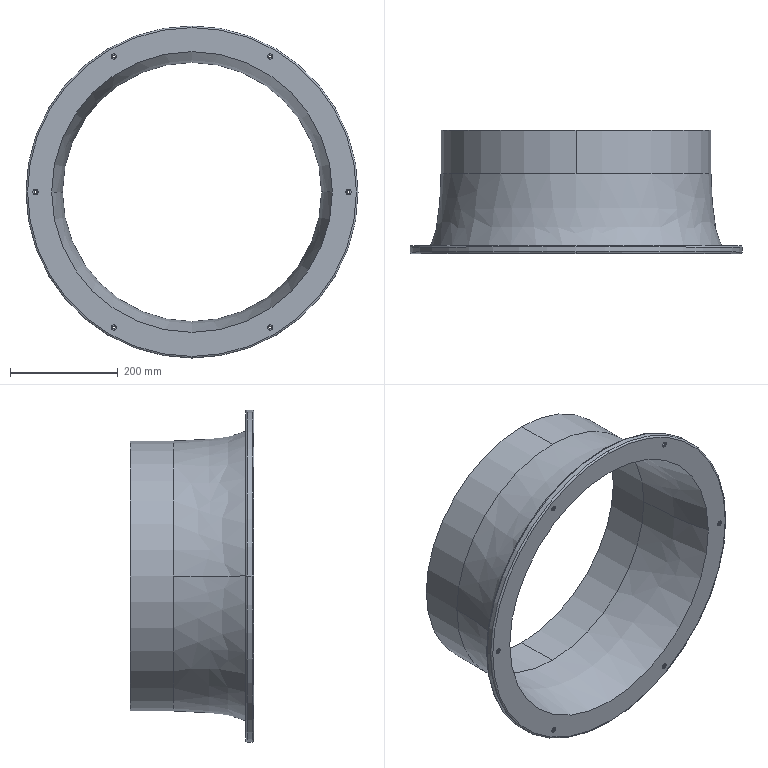Part | NX | features BREP 1 | 1 solid | 47 faces | box 615 x 228.661 x 615 mm | volume 4640014 mm3 | cylinder 30 | plane 9 | spline 4 | torus 4 | commonest cylinder face diameters 5 x12 10 x12 480 x2 500 x2 615 x2
STEP:
#1=CARTESIAN_POINT('',(0.,0.,-240.));
#2=VERTEX_POINT('',#1);
#3=CARTESIAN_POINT('',(-240.,0.,0.));
#4=VERTEX_POINT('',#3);
#5=CARTESIAN_POINT('',(0.,0.,0.));
#6=DIRECTION('',(0.,1.,0.));
#7=DIRECTION('',(0.,0.,1.));
#8=AXIS2_PLACEMENT_3D('',#5,#6,#7);
#9=CIRCLE('',#8,240.);
#10=EDGE_CURVE('',#2,#4,#9,.T.);
#11=ORIENTED_EDGE('',*,*,#10,.T.);
#12=CARTESIAN_POINT('',(-260.,-148.661,0.));
#13=VERTEX_POINT('',#12);
#14=CARTESIAN_POINT('',(-240.,0.,0.));
#15=CARTESIAN_POINT('',(-240.747,-21.775,0.));
#16=CARTESIAN_POINT('',(-242.819,-71.923,0.));
#17=CARTESIAN_POINT('',(-251.4,-121.567,0.));
#18=CARTESIAN_POINT('',(-260.,-148.661,0.));
#19=B_SPLINE_CURVE_WITH_KNOTS('',3,(#14,#15,#16,#17,#18),.UNSPECIFIED.,.F.,.F.,(4,1,4),(0.,0.4345,1.),.UNSPECIFIED.);
#20=EDGE_CURVE('',#4,#13,#19,.T.);
#21=ORIENTED_EDGE('',*,*,#20,.T.);
#22=CARTESIAN_POINT('',(260.,-148.661,0.));
#23=VERTEX_POINT('',#22);
#24=CARTESIAN_POINT('',(0.,-148.661,0.));
#25=DIRECTION('',(0.,1.,0.));
#26=DIRECTION('',(0.,0.,1.));
#27=AXIS2_PLACEMENT_3D('',#24,#25,#26);
#28=CIRCLE('',#27,260.);
#29=EDGE_CURVE('',#23,#13,#28,.T.);
#30=ORIENTED_EDGE('',*,*,#29,.F.);
#31=CARTESIAN_POINT('',(240.,0.,0.));
#32=VERTEX_POINT('',#31);
#33=CARTESIAN_POINT('',(240.,0.,0.));
#34=CARTESIAN_POINT('',(240.747,-21.775,0.));
#35=CARTESIAN_POINT('',(242.819,-71.923,0.));
#36=CARTESIAN_POINT('',(251.4,-121.567,0.));
#37=CARTESIAN_POINT('',(260.,-148.661,0.));
#38=B_SPLINE_CURVE_WITH_KNOTS('',3,(#33,#34,#35,#36,#37),.UNSPECIFIED.,.F.,.F.,(4,1,4),(0.,0.4345,1.),.UNSPECIFIED.);
#39=EDGE_CURVE('',#32,#23,#38,.T.);
#40=ORIENTED_EDGE('',*,*,#39,.F.);
#41=CARTESIAN_POINT('',(0.,0.,0.));
#42=DIRECTION('',(0.,1.,0.));
#43=DIRECTION('',(0.,0.,1.));
#44=AXIS2_PLACEMENT_3D('',#41,#42,#43);
#45=CIRCLE('',#44,240.);
#46=EDGE_CURVE('',#32,#2,#45,.T.);
#47=ORIENTED_EDGE('',*,*,#46,.T.);
#48=EDGE_LOOP('',(#11,#21,#30,#40,#47));
#49=FACE_BOUND('',#48,.T.);
#50=CARTESIAN_POINT('',(240.,0.,0.));
#51=CARTESIAN_POINT('',(240.,0.,-480.));
#52=CARTESIAN_POINT('',(-240.,0.,-480.));
#53=CARTESIAN_POINT('',(-240.,0.,0.));
#54=CARTESIAN_POINT('',(240.747,-21.775,0.));
#55=CARTESIAN_POINT('',(240.747,-21.775,-481.494));
#56=CARTESIAN_POINT('',(-240.747,-21.775,-481.494));
#57=CARTESIAN_POINT('',(-240.747,-21.775,0.));
#58=CARTESIAN_POINT('',(242.819,-71.923,0.));
#59=CARTESIAN_POINT('',(242.819,-71.923,-485.639));
#60=CARTESIAN_POINT('',(-242.819,-71.923,-485.639));
#61=CARTESIAN_POINT('',(-242.819,-71.923,0.));
#62=CARTESIAN_POINT('',(251.4,-121.567,0.));
#63=CARTESIAN_POINT('',(251.4,-121.567,-502.8));
#64=CARTESIAN_POINT('',(-251.4,-121.567,-502.8));
#65=CARTESIAN_POINT('',(-251.4,-121.567,0.));
#66=CARTESIAN_POINT('',(260.,-148.661,0.));
#67=CARTESIAN_POINT('',(260.,-148.661,-520.));
#68=CARTESIAN_POINT('',(-260.,-148.661,-520.));
#69=CARTESIAN_POINT('',(-260.,-148.661,0.));
#70=(BOUNDED_SURFACE()B_SPLINE_SURFACE(3,3,((#50,#51,#52,#53),(#54,#55,#56,#57),(#58,#59,#60,#61),(#62,#63,#64,#65),(#66,#67,#68,#69)),.SURF_OF_REVOLUTION.,.F.,.F.,.F.)B_SPLINE_SURFACE_WITH_KNOTS((4,1,4),(4,4),(0.,0.4345,1.),(0.,1.),.UNSPECIFIED.)GEOMETRIC_REPRESENTATION_ITEM()RATIONAL_B_SPLINE_SURFACE(((1.,0.3333,0.3333,1.),(1.,0.3333,0.3333,1.),(1.,0.3333,0.3333,1.),(1.,0.3333,0.3333,1.),(1.,0.3333,0.3333,1.)))REPRESENTATION_ITEM('')SURFACE());
#71=ADVANCED_FACE('',(#49),#70,.F.);
#72=CARTESIAN_POINT('',(-269.294,-133.661,0.));
#73=VERTEX_POINT('',#72);
#74=CARTESIAN_POINT('',(269.294,-133.661,0.));
#75=VERTEX_POINT('',#74);
#76=CARTESIAN_POINT('',(0.,-133.661,0.));
#77=DIRECTION('',(0.,-1.,0.));
#78=DIRECTION('',(0.,0.,1.));
#79=AXIS2_PLACEMENT_3D('',#76,#77,#78);
#80=CIRCLE('',#79,269.294);
#81=EDGE_CURVE('',#73,#75,#80,.T.);
#82=ORIENTED_EDGE('',*,*,#81,.F.);
#83=CARTESIAN_POINT('',(-250.,0.,0.));
#84=VERTEX_POINT('',#83);
#85=CARTESIAN_POINT('',(-269.294,-133.661,0.));
#86=CARTESIAN_POINT('',(-258.305,-112.435,0.));
#87=CARTESIAN_POINT('',(-252.887,-66.867,0.));
#88=CARTESIAN_POINT('',(-250.043,-21.856,0.));
#89=CARTESIAN_POINT('',(-250.,0.,0.));
#90=B_SPLINE_CURVE_WITH_KNOTS('',3,(#85,#86,#87,#88,#89),.UNSPECIFIED.,.F.,.F.,(4,1,4),(0.,0.5193,1.),.UNSPECIFIED.);
#91=EDGE_CURVE('',#73,#84,#90,.T.);
#92=ORIENTED_EDGE('',*,*,#91,.T.);
#93=CARTESIAN_POINT('',(0.,0.,-250.));
#94=VERTEX_POINT('',#93);
#95=CARTESIAN_POINT('',(0.,0.,0.));
#96=DIRECTION('',(0.,1.,0.));
#97=DIRECTION('',(0.,0.,1.));
#98=AXIS2_PLACEMENT_3D('',#95,#96,#97);
#99=CIRCLE('',#98,250.);
#100=EDGE_CURVE('',#94,#84,#99,.T.);
#101=ORIENTED_EDGE('',*,*,#100,.F.);
#102=CARTESIAN_POINT('',(250.,0.,0.));
#103=VERTEX_POINT('',#102);
#104=CARTESIAN_POINT('',(0.,0.,0.));
#105=DIRECTION('',(0.,1.,0.));
#106=DIRECTION('',(0.,0.,1.));
#107=AXIS2_PLACEMENT_3D('',#104,#105,#106);
#108=CIRCLE('',#107,250.);
#109=EDGE_CURVE('',#103,#94,#108,.T.);
#110=ORIENTED_EDGE('',*,*,#109,.F.);
#111=CARTESIAN_POINT('',(269.294,-133.661,0.));
#112=CARTESIAN_POINT('',(258.305,-112.435,0.));
#113=CARTESIAN_POINT('',(252.887,-66.867,0.));
#114=CARTESIAN_POINT('',(250.043,-21.856,0.));
#115=CARTESIAN_POINT('',(250.,0.,0.));
#116=B_SPLINE_CURVE_WITH_KNOTS('',3,(#111,#112,#113,#114,#115),.UNSPECIFIED.,.F.,.F.,(4,1,4),(0.,0.5193,1.),.UNSPECIFIED.);
#117=EDGE_CURVE('',#75,#103,#116,.T.);
#118=ORIENTED_EDGE('',*,*,#117,.F.);
#119=EDGE_LOOP('',(#82,#92,#101,#110,#118));
#120=FACE_BOUND('',#119,.T.);
#121=CARTESIAN_POINT('',(269.294,-133.661,0.));
#122=CARTESIAN_POINT('',(269.294,-133.661,-538.588));
#123=CARTESIAN_POINT('',(-269.294,-133.661,-538.588));
#124=CARTESIAN_POINT('',(-269.294,-133.661,0.));
#125=CARTESIAN_POINT('',(258.305,-112.435,0.));
#126=CARTESIAN_POINT('',(258.305,-112.435,-516.61));
#127=CARTESIAN_POINT('',(-258.305,-112.435,-516.61));
#128=CARTESIAN_POINT('',(-258.305,-112.435,0.));
#129=CARTESIAN_POINT('',(252.887,-66.867,0.));
#130=CARTESIAN_POINT('',(252.887,-66.867,-505.774));
#131=CARTESIAN_POINT('',(-252.887,-66.867,-505.774));
#132=CARTESIAN_POINT('',(-252.887,-66.867,0.));
#133=CARTESIAN_POINT('',(250.043,-21.856,0.));
#134=CARTESIAN_POINT('',(250.043,-21.856,-500.085));
#135=CARTESIAN_POINT('',(-250.043,-21.856,-500.085));
#136=CARTESIAN_POINT('',(-250.043,-21.856,0.));
#137=CARTESIAN_POINT('',(250.,0.,0.));
#138=CARTESIAN_POINT('',(250.,0.,-500.));
#139=CARTESIAN_POINT('',(-250.,0.,-500.));
#140=CARTESIAN_POINT('',(-250.,0.,0.));
#141=(BOUNDED_SURFACE()B_SPLINE_SURFACE(3,3,((#121,#122,#123,#124),(#125,#126,#127,#128),(#129,#130,#131,#132),(#133,#134,#135,#136),(#137,#138,#139,#140)),.SURF_OF_REVOLUTION.,.F.,.F.,.F.)B_SPLINE_SURFACE_WITH_KNOTS((4,1,4),(4,4),(0.,0.5193,1.),(0.,1.),.UNSPECIFIED.)GEOMETRIC_REPRESENTATION_ITEM()RATIONAL_B_SPLINE_SURFACE(((1.,0.3333,0.3333,1.),(1.,0.3333,0.3333,1.),(1.,0.3333,0.3333,1.),(1.,0.3333,0.3333,1.),(1.,0.3333,0.3333,1.)))REPRESENTATION_ITEM('')SURFACE());
#142=ADVANCED_FACE('',(#120),#141,.F.);
#143=CARTESIAN_POINT('',(-145.,-146.661,-246.147));
#144=VERTEX_POINT('',#143);
#145=CARTESIAN_POINT('',(-145.,-146.661,-256.147));
#146=VERTEX_POINT('',#145);
#147=CARTESIAN_POINT('',(-145.,-146.661,-251.147));
#148=DIRECTION('',(0.,-1.,0.));
#149=DIRECTION('',(0.866,0.,-0.5));
#150=AXIS2_PLACEMENT_3D('',#147,#148,#149);
#151=CIRCLE('',#150,5.);
#152=EDGE_CURVE('',#144,#146,#151,.T.);
#153=ORIENTED_EDGE('',*,*,#152,.F.);
#154=CARTESIAN_POINT('',(-145.,-148.661,-246.147));
#155=VERTEX_POINT('',#154);
#156=CARTESIAN_POINT('',(-145.,-146.661,-246.147));
#157=DIRECTION('',(0.,-1.,0.));
#158=VECTOR('',#157,1000.);
#159=LINE('',#156,#158);
#160=EDGE_CURVE('',#155,#144,#159,.F.);
#161=ORIENTED_EDGE('',*,*,#160,.F.);
#162=CARTESIAN_POINT('',(-145.,-148.661,-256.147));
#163=VERTEX_POINT('',#162);
#164=CARTESIAN_POINT('',(-145.,-148.661,-251.147));
#165=DIRECTION('',(0.,-1.,0.));
#166=DIRECTION('',(0.866,0.,-0.5));
#167=AXIS2_PLACEMENT_3D('',#164,#165,#166);
#168=CIRCLE('',#167,5.);
#169=EDGE_CURVE('',#155,#163,#168,.T.);
#170=ORIENTED_EDGE('',*,*,#169,.T.);
#171=CARTESIAN_POINT('',(-145.,-146.661,-256.147));
#172=DIRECTION('',(0.,-1.,0.));
#173=VECTOR('',#172,1000.);
#174=LINE('',#171,#173);
#175=EDGE_CURVE('',#163,#146,#174,.F.);
#176=ORIENTED_EDGE('',*,*,#175,.T.);
#177=EDGE_LOOP('',(#153,#161,#170,#176));
#178=FACE_BOUND('',#177,.T.);
#179=CARTESIAN_POINT('',(-145.,-146.661,-251.147));
#180=DIRECTION('',(0.,-1.,0.));
#181=DIRECTION('',(0.,0.,1.));
#182=AXIS2_PLACEMENT_3D('',#179,#180,#181);
#183=CYLINDRICAL_SURFACE('',#182,5.);
#184=ADVANCED_FACE('',(#178),#183,.F.);
#185=CARTESIAN_POINT('',(145.,-146.661,-246.147));
#186=VERTEX_POINT('',#185);
#187=CARTESIAN_POINT('',(145.,-146.661,-256.147));
#188=VERTEX_POINT('',#187);
#189=CARTESIAN_POINT('',(145.,-146.661,-251.147));
#190=DIRECTION('',(0.,-1.,0.));
#191=DIRECTION('',(0.866,0.,0.5));
#192=AXIS2_PLACEMENT_3D('',#189,#190,#191);
#193=CIRCLE('',#192,5.);
#194=EDGE_CURVE('',#186,#188,#193,.T.);
#195=ORIENTED_EDGE('',*,*,#194,.F.);
#196=CARTESIAN_POINT('',(145.,-148.661,-246.147));
#197=VERTEX_POINT('',#196);
#198=CARTESIAN_POINT('',(145.,-146.661,-246.147));
#199=DIRECTION('',(0.,-1.,0.));
#200=VECTOR('',#199,1000.);
#201=LINE('',#198,#200);
#202=EDGE_CURVE('',#197,#186,#201,.F.);
#203=ORIENTED_EDGE('',*,*,#202,.F.);
#204=CARTESIAN_POINT('',(145.,-148.661,-256.147));
#205=VERTEX_POINT('',#204);
#206=CARTESIAN_POINT('',(145.,-148.661,-251.147));
#207=DIRECTION('',(0.,-1.,0.));
#208=DIRECTION('',(0.866,0.,0.5));
#209=AXIS2_PLACEMENT_3D('',#206,#207,#208);
#210=CIRCLE('',#209,5.);
#211=EDGE_CURVE('',#197,#205,#210,.T.);
#212=ORIENTED_EDGE('',*,*,#211,.T.);
#213=CARTESIAN_POINT('',(145.,-146.661,-256.147));
#214=DIRECTION('',(0.,-1.,0.));
#215=VECTOR('',#214,1000.);
#216=LINE('',#213,#215);
#217=EDGE_CURVE('',#205,#188,#216,.F.);
#218=ORIENTED_EDGE('',*,*,#217,.T.);
#219=EDGE_LOOP('',(#195,#203,#212,#218));
#220=FACE_BOUND('',#219,.T.);
#221=CARTESIAN_POINT('',(145.,-146.661,-251.147));
#222=DIRECTION('',(0.,-1.,0.));
#223=DIRECTION('',(0.,0.,1.));
#224=AXIS2_PLACEMENT_3D('',#221,#222,#223);
#225=CYLINDRICAL_SURFACE('',#224,5.);
#226=ADVANCED_FACE('',(#220),#225,.F.);
#227=CARTESIAN_POINT('',(290.,-146.661,5.));
#228=VERTEX_POINT('',#227);
#229=CARTESIAN_POINT('',(290.,-146.661,-5.));
#230=VERTEX_POINT('',#229);
#231=CARTESIAN_POINT('',(290.,-146.661,0.));
#232=DIRECTION('',(0.,-1.,0.));
#233=DIRECTION('',(0.,0.,1.));
#234=AXIS2_PLACEMENT_3D('',#231,#232,#233);
#235=CIRCLE('',#234,5.);
#236=EDGE_CURVE('',#228,#230,#235,.T.);
#237=ORIENTED_EDGE('',*,*,#236,.F.);
#238=CARTESIAN_POINT('',(290.,-148.661,5.));
#239=VERTEX_POINT('',#238);
#240=CARTESIAN_POINT('',(290.,-146.661,5.));
#241=DIRECTION('',(0.,-1.,0.));
#242=VECTOR('',#241,1000.);
#243=LINE('',#240,#242);
#244=EDGE_CURVE('',#239,#228,#243,.F.);
#245=ORIENTED_EDGE('',*,*,#244,.F.);
#246=CARTESIAN_POINT('',(290.,-148.661,-5.));
#247=VERTEX_POINT('',#246);
#248=CARTESIAN_POINT('',(290.,-148.661,0.));
#249=DIRECTION('',(0.,-1.,0.));
#250=DIRECTION('',(0.,0.,1.));
#251=AXIS2_PLACEMENT_3D('',#248,#249,#250);
#252=CIRCLE('',#251,5.);
#253=EDGE_CURVE('',#239,#247,#252,.T.);
#254=ORIENTED_EDGE('',*,*,#253,.T.);
#255=CARTESIAN_POINT('',(290.,-146.661,-5.));
#256=DIRECTION('',(0.,-1.,0.));
#257=VECTOR('',#256,1000.);
#258=LINE('',#255,#257);
#259=EDGE_CURVE('',#247,#230,#258,.F.);
#260=ORIENTED_EDGE('',*,*,#259,.T.);
#261=EDGE_LOOP('',(#237,#245,#254,#260));
#262=FACE_BOUND('',#261,.T.);
#263=CARTESIAN_POINT('',(290.,-146.661,0.));
#264=DIRECTION('',(0.,-1.,0.));
#265=DIRECTION('',(0.,0.,1.));
#266=AXIS2_PLACEMENT_3D('',#263,#264,#265);
#267=CYLINDRICAL_SURFACE('',#266,5.);
#268=ADVANCED_FACE('',(#262),#267,.F.);
#269=CARTESIAN_POINT('',(145.,-146.661,256.147));
#270=VERTEX_POINT('',#269);
#271=CARTESIAN_POINT('',(145.,-146.661,246.147));
#272=VERTEX_POINT('',#271);
#273=CARTESIAN_POINT('',(145.,-146.661,251.147));
#274=DIRECTION('',(0.,-1.,0.));
#275=DIRECTION('',(-0.866,0.,0.5));
#276=AXIS2_PLACEMENT_3D('',#273,#274,#275);
#277=CIRCLE('',#276,5.);
#278=EDGE_CURVE('',#270,#272,#277,.T.);
#279=ORIENTED_EDGE('',*,*,#278,.F.);
#280=CARTESIAN_POINT('',(145.,-148.661,256.147));
#281=VERTEX_POINT('',#280);
#282=CARTESIAN_POINT('',(145.,-146.661,256.147));
#283=DIRECTION('',(0.,-1.,0.));
#284=VECTOR('',#283,1000.);
#285=LINE('',#282,#284);
#286=EDGE_CURVE('',#281,#270,#285,.F.);
#287=ORIENTED_EDGE('',*,*,#286,.F.);
#288=CARTESIAN_POINT('',(145.,-148.661,246.147));
#289=VERTEX_POINT('',#288);
#290=CARTESIAN_POINT('',(145.,-148.661,251.147));
#291=DIRECTION('',(0.,-1.,0.));
#292=DIRECTION('',(-0.866,0.,0.5));
#293=AXIS2_PLACEMENT_3D('',#290,#291,#292);
#294=CIRCLE('',#293,5.);
#295=EDGE_CURVE('',#281,#289,#294,.T.);
#296=ORIENTED_EDGE('',*,*,#295,.T.);
#297=CARTESIAN_POINT('',(145.,-146.661,246.147));
#298=DIRECTION('',(0.,-1.,0.));
#299=VECTOR('',#298,1000.);
#300=LINE('',#297,#299);
#301=EDGE_CURVE('',#289,#272,#300,.F.);
#302=ORIENTED_EDGE('',*,*,#301,.T.);
#303=EDGE_LOOP('',(#279,#287,#296,#302));
#304=FACE_BOUND('',#303,.T.);
#305=CARTESIAN_POINT('',(145.,-146.661,251.147));
#306=DIRECTION('',(0.,-1.,0.));
#307=DIRECTION('',(0.,0.,1.));
#308=AXIS2_PLACEMENT_3D('',#305,#306,#307);
#309=CYLINDRICAL_SURFACE('',#308,5.);
#310=ADVANCED_FACE('',(#304),#309,.F.);
#311=CARTESIAN_POINT('',(-145.,-146.661,256.147));
#312=VERTEX_POINT('',#311);
#313=CARTESIAN_POINT('',(-145.,-146.661,246.147));
#314=VERTEX_POINT('',#313);
#315=CARTESIAN_POINT('',(-145.,-146.661,251.147));
#316=DIRECTION('',(0.,-1.,0.));
#317=DIRECTION('',(-0.866,0.,-0.5));
#318=AXIS2_PLACEMENT_3D('',#315,#316,#317);
#319=CIRCLE('',#318,5.);
#320=EDGE_CURVE('',#312,#314,#319,.T.);
#321=ORIENTED_EDGE('',*,*,#320,.F.);
#322=CARTESIAN_POINT('',(-145.,-148.661,256.147));
#323=VERTEX_POINT('',#322);
#324=CARTESIAN_POINT('',(-145.,-146.661,256.147));
#325=DIRECTION('',(0.,-1.,0.));
#326=VECTOR('',#325,1000.);
#327=LINE('',#324,#326);
#328=EDGE_CURVE('',#323,#312,#327,.F.);
#329=ORIENTED_EDGE('',*,*,#328,.F.);
#330=CARTESIAN_POINT('',(-145.,-148.661,246.147));
#331=VERTEX_POINT('',#330);
#332=CARTESIAN_POINT('',(-145.,-148.661,251.147));
#333=DIRECTION('',(0.,-1.,0.));
#334=DIRECTION('',(-0.866,0.,-0.5));
#335=AXIS2_PLACEMENT_3D('',#332,#333,#334);
#336=CIRCLE('',#335,5.);
#337=EDGE_CURVE('',#323,#331,#336,.T.);
#338=ORIENTED_EDGE('',*,*,#337,.T.);
#339=CARTESIAN_POINT('',(-145.,-146.661,246.147));
#340=DIRECTION('',(0.,-1.,0.));
#341=VECTOR('',#340,1000.);
#342=LINE('',#339,#341);
#343=EDGE_CURVE('',#331,#314,#342,.F.);
#344=ORIENTED_EDGE('',*,*,#343,.T.);
#345=EDGE_LOOP('',(#321,#329,#338,#344));
#346=FACE_BOUND('',#345,.T.);
#347=CARTESIAN_POINT('',(-145.,-146.661,251.147));
#348=DIRECTION('',(0.,-1.,0.));
#349=DIRECTION('',(0.,0.,1.));
#350=AXIS2_PLACEMENT_3D('',#347,#348,#349);
#351=CYLINDRICAL_SURFACE('',#350,5.);
#352=ADVANCED_FACE('',(#346),#351,.F.);
#353=CARTESIAN_POINT('',(-290.,-146.661,5.));
#354=VERTEX_POINT('',#353);
#355=CARTESIAN_POINT('',(-290.,-146.661,-5.));
#356=VERTEX_POINT('',#355);
#357=CARTESIAN_POINT('',(-290.,-146.661,0.));
#358=DIRECTION('',(0.,-1.,0.));
#359=DIRECTION('',(0.,0.,-1.));
#360=AXIS2_PLACEMENT_3D('',#357,#358,#359);
#361=CIRCLE('',#360,5.);
#362=EDGE_CURVE('',#354,#356,#361,.T.);
#363=ORIENTED_EDGE('',*,*,#362,.F.);
#364=CARTESIAN_POINT('',(-290.,-148.661,5.));
#365=VERTEX_POINT('',#364);
#366=CARTESIAN_POINT('',(-290.,-146.661,5.));
#367=DIRECTION('',(0.,-1.,0.));
#368=VECTOR('',#367,1000.);
#369=LINE('',#366,#368);
#370=EDGE_CURVE('',#365,#354,#369,.F.);
#371=ORIENTED_EDGE('',*,*,#370,.F.);
#372=CARTESIAN_POINT('',(-290.,-148.661,-5.));
#373=VERTEX_POINT('',#372);
#374=CARTESIAN_POINT('',(-290.,-148.661,0.));
#375=DIRECTION('',(0.,-1.,0.));
#376=DIRECTION('',(0.,0.,-1.));
#377=AXIS2_PLACEMENT_3D('',#374,#375,#376);
#378=CIRCLE('',#377,5.);
#379=EDGE_CURVE('',#365,#373,#378,.T.);
#380=ORIENTED_EDGE('',*,*,#379,.T.);
#381=CARTESIAN_POINT('',(-290.,-146.661,-5.));
#382=DIRECTION('',(0.,-1.,0.));
#383=VECTOR('',#382,1000.);
#384=LINE('',#381,#383);
#385=EDGE_CURVE('',#373,#356,#384,.F.);
#386=ORIENTED_EDGE('',*,*,#385,.T.);
#387=EDGE_LOOP('',(#363,#371,#380,#386));
#388=FACE_BOUND('',#387,.T.);
#389=CARTESIAN_POINT('',(-290.,-146.661,0.));
#390=DIRECTION('',(0.,-1.,0.));
#391=DIRECTION('',(0.,0.,1.));
#392=AXIS2_PLACEMENT_3D('',#389,#390,#391);
#393=CYLINDRICAL_SURFACE('',#392,5.);
#394=ADVANCED_FACE('',(#388),#393,.F.);
#395=CARTESIAN_POINT('',(-304.5,-133.661,0.));
#396=VERTEX_POINT('',#395);
#397=CARTESIAN_POINT('',(304.5,-133.661,0.));
#398=VERTEX_POINT('',#397);
#399=CARTESIAN_POINT('',(0.,-133.661,0.));
#400=DIRECTION('',(0.,1.,0.));
#401=DIRECTION('',(1.,0.,0.));
#402=AXIS2_PLACEMENT_3D('',#399,#400,#401);
#403=CIRCLE('',#402,304.5);
#404=EDGE_CURVE('',#396,#398,#403,.T.);
#405=ORIENTED_EDGE('',*,*,#404,.F.);
#406=CARTESIAN_POINT('',(-307.5,-136.661,0.));
#407=VERTEX_POINT('',#406);
#408=CARTESIAN_POINT('',(-304.5,-136.661,0.));
#409=DIRECTION('',(0.,0.,1.));
#410=DIRECTION('',(1.,0.,0.));
#411=AXIS2_PLACEMENT_3D('',#408,#409,#410);
#412=CIRCLE('',#411,3.);
#413=EDGE_CURVE('',#396,#407,#412,.T.);
#414=ORIENTED_EDGE('',*,*,#413,.T.);
#415=CARTESIAN_POINT('',(307.5,-136.661,0.));
#416=VERTEX_POINT('',#415);
#417=CARTESIAN_POINT('',(0.,-136.661,0.));
#418=DIRECTION('',(0.,-1.,0.));
#419=DIRECTION('',(1.,0.,0.));
#420=AXIS2_PLACEMENT_3D('',#417,#418,#419);
#421=CIRCLE('',#420,307.5);
#422=EDGE_CURVE('',#416,#407,#421,.T.);
#423=ORIENTED_EDGE('',*,*,#422,.F.);
#424=CARTESIAN_POINT('',(304.5,-136.661,0.));
#425=DIRECTION('',(0.,0.,-1.));
#426=DIRECTION('',(-1.,0.,0.));
#427=AXIS2_PLACEMENT_3D('',#424,#425,#426);
#428=CIRCLE('',#427,3.);
#429=EDGE_CURVE('',#398,#416,#428,.T.);
#430=ORIENTED_EDGE('',*,*,#429,.F.);
#431=EDGE_LOOP('',(#405,#414,#423,#430));
#432=FACE_BOUND('',#431,.T.);
#433=CARTESIAN_POINT('',(0.,-136.661,0.));
#434=DIRECTION('',(0.,-1.,0.));
#435=DIRECTION('',(-1.,0.,0.));
#436=AXIS2_PLACEMENT_3D('',#433,#434,#435);
#437=TOROIDAL_SURFACE('',#436,304.5,3.);
#438=ADVANCED_FACE('',(#432),#437,.T.);
#439=CARTESIAN_POINT('',(0.,-148.661,-304.5));
#440=VERTEX_POINT('',#439);
#441=CARTESIAN_POINT('',(0.,-148.661,304.5));
#442=VERTEX_POINT('',#441);
#443=CARTESIAN_POINT('',(0.,-148.661,0.));
#444=DIRECTION('',(0.,-1.,0.));
#445=DIRECTION('',(0.,0.,1.));
#446=AXIS2_PLACEMENT_3D('',#443,#444,#445);
#447=CIRCLE('',#446,304.5);
#448=EDGE_CURVE('',#440,#442,#447,.T.);
#449=ORIENTED_EDGE('',*,*,#448,.F.);
#450=CARTESIAN_POINT('',(0.,-145.661,-307.5));
#451=VERTEX_POINT('',#450);
#452=CARTESIAN_POINT('',(0.,-145.661,-304.5));
#453=DIRECTION('',(1.,0.,0.));
#454=DIRECTION('',(0.,0.,-1.));
#455=AXIS2_PLACEMENT_3D('',#452,#453,#454);
#456=CIRCLE('',#455,3.);
#457=EDGE_CURVE('',#440,#451,#456,.T.);
#458=ORIENTED_EDGE('',*,*,#457,.T.);
#459=CARTESIAN_POINT('',(307.5,-145.661,0.));
#460=VERTEX_POINT('',#459);
#461=CARTESIAN_POINT('',(0.,-145.661,0.));
#462=DIRECTION('',(0.,1.,0.));
#463=DIRECTION('',(0.,0.,1.));
#464=AXIS2_PLACEMENT_3D('',#461,#462,#463);
#465=CIRCLE('',#464,307.5);
#466=EDGE_CURVE('',#460,#451,#465,.T.);
#467=ORIENTED_EDGE('',*,*,#466,.F.);
#468=CARTESIAN_POINT('',(0.,-145.661,307.5));
#469=VERTEX_POINT('',#468);
#470=CARTESIAN_POINT('',(0.,-145.661,0.));
#471=DIRECTION('',(0.,1.,0.));
#472=DIRECTION('',(0.,0.,1.));
#473=AXIS2_PLACEMENT_3D('',#470,#471,#472);
#474=CIRCLE('',#473,307.5);
#475=EDGE_CURVE('',#469,#460,#474,.T.);
#476=ORIENTED_EDGE('',*,*,#475,.F.);
#477=CARTESIAN_POINT('',(0.,-145.661,304.5));
#478=DIRECTION('',(-1.,0.,0.));
#479=DIRECTION('',(0.,0.,1.));
#480=AXIS2_PLACEMENT_3D('',#477,#478,#479);
#481=CIRCLE('',#480,3.);
#482=EDGE_CURVE('',#442,#469,#481,.T.);
#483=ORIENTED_EDGE('',*,*,#482,.F.);
#484=EDGE_LOOP('',(#449,#458,#467,#476,#483));
#485=FACE_BOUND('',#484,.T.);
#486=CARTESIAN_POINT('',(0.,-145.661,0.));
#487=DIRECTION('',(0.,1.,0.));
#488=DIRECTION('',(0.,0.,-1.));
#489=AXIS2_PLACEMENT_3D('',#486,#487,#488);
#490=TOROIDAL_SURFACE('',#489,304.5,3.);
#491=ADVANCED_FACE('',(#485),#490,.T.);
#492=ORIENTED_EDGE('',*,*,#422,.T.);
#493=CARTESIAN_POINT('',(-307.5,-145.661,0.));
#494=VERTEX_POINT('',#493);
#495=CARTESIAN_POINT('',(-307.5,-133.661,0.));
#496=DIRECTION('',(0.,-1.,0.));
#497=VECTOR('',#496,1000.);
#498=LINE('',#495,#497);
#499=EDGE_CURVE('',#407,#494,#498,.T.);
#500=ORIENTED_EDGE('',*,*,#499,.T.);
#501=CARTESIAN_POINT('',(0.,-145.661,0.));
#502=DIRECTION('',(0.,1.,0.));
#503=DIRECTION('',(0.,0.,1.));
#504=AXIS2_PLACEMENT_3D('',#501,#502,#503);
#505=CIRCLE('',#504,307.5);
#506=EDGE_CURVE('',#494,#469,#505,.T.);
#507=ORIENTED_EDGE('',*,*,#506,.T.);
#508=ORIENTED_EDGE('',*,*,#475,.T.);
#509=CARTESIAN_POINT('',(307.5,-133.661,0.));
#510=DIRECTION('',(0.,-1.,0.));
#511=VECTOR('',#510,1000.);
#512=LINE('',#509,#511);
#513=EDGE_CURVE('',#416,#460,#512,.T.);
#514=ORIENTED_EDGE('',*,*,#513,.F.);
#515=EDGE_LOOP('',(#492,#500,#507,#508,#514));
#516=FACE_BOUND('',#515,.T.);
#517=CARTESIAN_POINT('',(0.,-133.661,0.));
#518=DIRECTION('',(0.,-1.,0.));
#519=DIRECTION('',(-1.,0.,0.));
#520=AXIS2_PLACEMENT_3D('',#517,#518,#519);
#521=CYLINDRICAL_SURFACE('',#520,307.5);
#522=ADVANCED_FACE('',(#516),#521,.T.);
#523=ORIENTED_EDGE('',*,*,#10,.F.);
#524=CARTESIAN_POINT('',(0.,80.,-240.));
#525=VERTEX_POINT('',#524);
#526=CARTESIAN_POINT('',(0.,0.,-240.));
#527=DIRECTION('',(0.,1.,0.));
#528=VECTOR('',#527,1000.);
#529=LINE('',#526,#528);
#530=EDGE_CURVE('',#2,#525,#529,.T.);
#531=ORIENTED_EDGE('',*,*,#530,.T.);
#532=CARTESIAN_POINT('',(0.,80.,240.));
#533=VERTEX_POINT('',#532);
#534=CARTESIAN_POINT('',(0.,80.,0.));
#535=DIRECTION('',(0.,1.,0.));
#536=DIRECTION('',(0.,0.,1.));
#537=AXIS2_PLACEMENT_3D('',#534,#535,#536);
#538=CIRCLE('',#537,240.);
#539=EDGE_CURVE('',#525,#533,#538,.T.);
#540=ORIENTED_EDGE('',*,*,#539,.T.);
#541=CARTESIAN_POINT('',(0.,0.,240.));
#542=VERTEX_POINT('',#541);
#543=CARTESIAN_POINT('',(0.,0.,240.));
#544=DIRECTION('',(0.,1.,0.));
#545=VECTOR('',#544,1000.);
#546=LINE('',#543,#545);
#547=EDGE_CURVE('',#542,#533,#546,.T.);
#548=ORIENTED_EDGE('',*,*,#547,.F.);
#549=CARTESIAN_POINT('',(0.,0.,0.));
#550=DIRECTION('',(0.,1.,0.));
#551=DIRECTION('',(0.,0.,1.));
#552=AXIS2_PLACEMENT_3D('',#549,#550,#551);
#553=CIRCLE('',#552,240.);
#554=EDGE_CURVE('',#4,#542,#553,.T.);
#555=ORIENTED_EDGE('',*,*,#554,.F.);
#556=EDGE_LOOP('',(#523,#531,#540,#548,#555));
#557=FACE_BOUND('',#556,.T.);
#558=CARTESIAN_POINT('',(0.,0.,0.));
#559=DIRECTION('',(0.,1.,0.));
#560=DIRECTION('',(0.,0.,-1.));
#561=AXIS2_PLACEMENT_3D('',#558,#559,#560);
#562=CYLINDRICAL_SURFACE('',#561,240.);
#563=ADVANCED_FACE('',(#557),#562,.F.);
#564=CARTESIAN_POINT('',(0.,0.,250.));
#565=VERTEX_POINT('',#564);
#566=CARTESIAN_POINT('',(0.,0.,0.));
#567=DIRECTION('',(0.,1.,0.));
#568=DIRECTION('',(0.,0.,1.));
#569=AXIS2_PLACEMENT_3D('',#566,#567,#568);
#570=CIRCLE('',#569,250.);
#571=EDGE_CURVE('',#565,#103,#570,.T.);
#572=ORIENTED_EDGE('',*,*,#571,.T.);
#573=ORIENTED_EDGE('',*,*,#109,.T.);
#574=CARTESIAN_POINT('',(0.,80.,-250.));
#575=VERTEX_POINT('',#574);
#576=CARTESIAN_POINT('',(0.,0.,-250.));
#577=DIRECTION('',(0.,1.,0.));
#578=VECTOR('',#577,1000.);
#579=LINE('',#576,#578);
#580=EDGE_CURVE('',#94,#575,#579,.T.);
#581=ORIENTED_EDGE('',*,*,#580,.T.);
#582=CARTESIAN_POINT('',(0.,80.,250.));
#583=VERTEX_POINT('',#582);
#584=CARTESIAN_POINT('',(0.,80.,0.));
#585=DIRECTION('',(0.,1.,0.));
#586=DIRECTION('',(0.,0.,1.));
#587=AXIS2_PLACEMENT_3D('',#584,#585,#586);
#588=CIRCLE('',#587,250.);
#589=EDGE_CURVE('',#583,#575,#588,.T.);
#590=ORIENTED_EDGE('',*,*,#589,.F.);
#591=CARTESIAN_POINT('',(0.,0.,250.));
#592=DIRECTION('',(0.,1.,0.));
#593=VECTOR('',#592,1000.);
#594=LINE('',#591,#593);
#595=EDGE_CURVE('',#565,#583,#594,.T.);
#596=ORIENTED_EDGE('',*,*,#595,.F.);
#597=EDGE_LOOP('',(#572,#573,#581,#590,#596));
#598=FACE_BOUND('',#597,.T.);
#599=CARTESIAN_POINT('',(0.,0.,0.));
#600=DIRECTION('',(0.,1.,0.));
#601=DIRECTION('',(0.,0.,-1.));
#602=AXIS2_PLACEMENT_3D('',#599,#600,#601);
#603=CYLINDRICAL_SURFACE('',#602,250.);
#604=ADVANCED_FACE('',(#598),#603,.T.);
#605=CARTESIAN_POINT('',(-292.5,-133.661,0.));
#606=VERTEX_POINT('',#605);
#607=CARTESIAN_POINT('',(-287.5,-133.661,0.));
#608=VERTEX_POINT('',#607);
#609=CARTESIAN_POINT('',(-290.,-133.661,0.));
#610=DIRECTION('',(0.,-1.,0.));
#611=DIRECTION('',(1.,0.,0.));
#612=AXIS2_PLACEMENT_3D('',#609,#610,#611);
#613=CIRCLE('',#612,2.5);
#614=EDGE_CURVE('',#606,#608,#613,.T.);
#615=ORIENTED_EDGE('',*,*,#614,.F.);
#616=CARTESIAN_POINT('',(-292.5,-146.661,0.));
#617=VERTEX_POINT('',#616);
#618=CARTESIAN_POINT('',(-292.5,-128.661,0.));
#619=DIRECTION('',(0.,-1.,0.));
#620=VECTOR('',#619,1000.);
#621=LINE('',#618,#620);
#622=EDGE_CURVE('',#606,#617,#621,.T.);
#623=ORIENTED_EDGE('',*,*,#622,.T.);
#624=CARTESIAN_POINT('',(-287.5,-146.661,0.));
#625=VERTEX_POINT('',#624);
#626=CARTESIAN_POINT('',(-290.,-146.661,0.));
#627=DIRECTION('',(0.,1.,0.));
#628=DIRECTION('',(0.,0.,-1.));
#629=AXIS2_PLACEMENT_3D('',#626,#627,#628);
#630=CIRCLE('',#629,2.5);
#631=EDGE_CURVE('',#625,#617,#630,.T.);
#632=ORIENTED_EDGE('',*,*,#631,.F.);
#633=CARTESIAN_POINT('',(-287.5,-128.661,0.));
#634=DIRECTION('',(0.,-1.,0.));
#635=VECTOR('',#634,1000.);
#636=LINE('',#633,#635);
#637=EDGE_CURVE('',#608,#625,#636,.T.);
#638=ORIENTED_EDGE('',*,*,#637,.F.);
#639=EDGE_LOOP('',(#615,#623,#632,#638));
#640=FACE_BOUND('',#639,.T.);
#641=CARTESIAN_POINT('',(-290.,-128.661,0.));
#642=DIRECTION('',(0.,-1.,0.));
#643=DIRECTION('',(-1.,0.,0.));
#644=AXIS2_PLACEMENT_3D('',#641,#642,#643);
#645=CYLINDRICAL_SURFACE('',#644,2.5);
#646=ADVANCED_FACE('',(#640),#645,.F.);
#647=CARTESIAN_POINT('',(-147.5,-133.661,251.147));
#648=VERTEX_POINT('',#647);
#649=CARTESIAN_POINT('',(-142.5,-133.661,251.147));
#650=VERTEX_POINT('',#649);
#651=CARTESIAN_POINT('',(-145.,-133.661,251.147));
#652=DIRECTION('',(0.,-1.,0.));
#653=DIRECTION('',(1.,0.,0.));
#654=AXIS2_PLACEMENT_3D('',#651,#652,#653);
#655=CIRCLE('',#654,2.5);
#656=EDGE_CURVE('',#648,#650,#655,.T.);
#657=ORIENTED_EDGE('',*,*,#656,.F.);
#658=CARTESIAN_POINT('',(-147.5,-146.661,251.147));
#659=VERTEX_POINT('',#658);
#660=CARTESIAN_POINT('',(-147.5,-128.661,251.147));
#661=DIRECTION('',(0.,-1.,0.));
#662=VECTOR('',#661,1000.);
#663=LINE('',#660,#662);
#664=EDGE_CURVE('',#648,#659,#663,.T.);
#665=ORIENTED_EDGE('',*,*,#664,.T.);
#666=CARTESIAN_POINT('',(-142.5,-146.661,251.147));
#667=VERTEX_POINT('',#666);
#668=CARTESIAN_POINT('',(-145.,-146.661,251.147));
#669=DIRECTION('',(0.,1.,0.));
#670=DIRECTION('',(0.,0.,-1.));
#671=AXIS2_PLACEMENT_3D('',#668,#669,#670);
#672=CIRCLE('',#671,2.5);
#673=EDGE_CURVE('',#667,#659,#672,.T.);
#674=ORIENTED_EDGE('',*,*,#673,.F.);
#675=CARTESIAN_POINT('',(-142.5,-128.661,251.147));
#676=DIRECTION('',(0.,-1.,0.));
#677=VECTOR('',#676,1000.);
#678=LINE('',#675,#677);
#679=EDGE_CURVE('',#650,#667,#678,.T.);
#680=ORIENTED_EDGE('',*,*,#679,.F.);
#681=EDGE_LOOP('',(#657,#665,#674,#680));
#682=FACE_BOUND('',#681,.T.);
#683=CARTESIAN_POINT('',(-145.,-128.661,251.147));
#684=DIRECTION('',(0.,-1.,0.));
#685=DIRECTION('',(-1.,0.,0.));
#686=AXIS2_PLACEMENT_3D('',#683,#684,#685);
#687=CYLINDRICAL_SURFACE('',#686,2.5);
#688=ADVANCED_FACE('',(#682),#687,.F.);
#689=CARTESIAN_POINT('',(142.5,-133.661,251.147));
#690=VERTEX_POINT('',#689);
#691=CARTESIAN_POINT('',(147.5,-133.661,251.147));
#692=VERTEX_POINT('',#691);
#693=CARTESIAN_POINT('',(145.,-133.661,251.147));
#694=DIRECTION('',(0.,-1.,0.));
#695=DIRECTION('',(1.,0.,0.));
#696=AXIS2_PLACEMENT_3D('',#693,#694,#695);
#697=CIRCLE('',#696,2.5);
#698=EDGE_CURVE('',#690,#692,#697,.T.);
#699=ORIENTED_EDGE('',*,*,#698,.F.);
#700=CARTESIAN_POINT('',(142.5,-146.661,251.147));
#701=VERTEX_POINT('',#700);
#702=CARTESIAN_POINT('',(142.5,-128.661,251.147));
#703=DIRECTION('',(0.,-1.,0.));
#704=VECTOR('',#703,1000.);
#705=LINE('',#702,#704);
#706=EDGE_CURVE('',#690,#701,#705,.T.);
#707=ORIENTED_EDGE('',*,*,#706,.T.);
#708=CARTESIAN_POINT('',(147.5,-146.661,251.147));
#709=VERTEX_POINT('',#708);
#710=CARTESIAN_POINT('',(145.,-146.661,251.147));
#711=DIRECTION('',(0.,1.,0.));
#712=DIRECTION('',(0.,0.,-1.));
#713=AXIS2_PLACEMENT_3D('',#710,#711,#712);
#714=CIRCLE('',#713,2.5);
#715=EDGE_CURVE('',#709,#701,#714,.T.);
#716=ORIENTED_EDGE('',*,*,#715,.F.);
#717=CARTESIAN_POINT('',(147.5,-128.661,251.147));
#718=DIRECTION('',(0.,-1.,0.));
#719=VECTOR('',#718,1000.);
#720=LINE('',#717,#719);
#721=EDGE_CURVE('',#692,#709,#720,.T.);
#722=ORIENTED_EDGE('',*,*,#721,.F.);
#723=EDGE_LOOP('',(#699,#707,#716,#722));
#724=FACE_BOUND('',#723,.T.);
#725=CARTESIAN_POINT('',(145.,-128.661,251.147));
#726=DIRECTION('',(0.,-1.,0.));
#727=DIRECTION('',(-1.,0.,0.));
#728=AXIS2_PLACEMENT_3D('',#725,#726,#727);
#729=CYLINDRICAL_SURFACE('',#728,2.5);
#730=ADVANCED_FACE('',(#724),#729,.F.);
#731=CARTESIAN_POINT('',(287.5,-133.661,0.));
#732=VERTEX_POINT('',#731);
#733=CARTESIAN_POINT('',(292.5,-133.661,0.));
#734=VERTEX_POINT('',#733);
#735=CARTESIAN_POINT('',(290.,-133.661,0.));
#736=DIRECTION('',(0.,-1.,0.));
#737=DIRECTION('',(1.,0.,0.));
#738=AXIS2_PLACEMENT_3D('',#735,#736,#737);
#739=CIRCLE('',#738,2.5);
#740=EDGE_CURVE('',#732,#734,#739,.T.);
#741=ORIENTED_EDGE('',*,*,#740,.F.);
#742=CARTESIAN_POINT('',(287.5,-146.661,0.));
#743=VERTEX_POINT('',#742);
#744=CARTESIAN_POINT('',(287.5,-128.661,0.));
#745=DIRECTION('',(0.,-1.,0.));
#746=VECTOR('',#745,1000.);
#747=LINE('',#744,#746);
#748=EDGE_CURVE('',#732,#743,#747,.T.);
#749=ORIENTED_EDGE('',*,*,#748,.T.);
#750=CARTESIAN_POINT('',(292.5,-146.661,0.));
#751=VERTEX_POINT('',#750);
#752=CARTESIAN_POINT('',(290.,-146.661,0.));
#753=DIRECTION('',(0.,1.,0.));
#754=DIRECTION('',(0.,0.,-1.));
#755=AXIS2_PLACEMENT_3D('',#752,#753,#754);
#756=CIRCLE('',#755,2.5);
#757=EDGE_CURVE('',#751,#743,#756,.T.);
#758=ORIENTED_EDGE('',*,*,#757,.F.);
#759=CARTESIAN_POINT('',(292.5,-128.661,0.));
#760=DIRECTION('',(0.,-1.,0.));
#761=VECTOR('',#760,1000.);
#762=LINE('',#759,#761);
#763=EDGE_CURVE('',#734,#751,#762,.T.);
#764=ORIENTED_EDGE('',*,*,#763,.F.);
#765=EDGE_LOOP('',(#741,#749,#758,#764));
#766=FACE_BOUND('',#765,.T.);
#767=CARTESIAN_POINT('',(290.,-128.661,0.));
#768=DIRECTION('',(0.,-1.,0.));
#769=DIRECTION('',(-1.,0.,0.));
#770=AXIS2_PLACEMENT_3D('',#767,#768,#769);
#771=CYLINDRICAL_SURFACE('',#770,2.5);
#772=ADVANCED_FACE('',(#766),#771,.F.);
#773=CARTESIAN_POINT('',(142.5,-133.661,-251.147));
#774=VERTEX_POINT('',#773);
#775=CARTESIAN_POINT('',(147.5,-133.661,-251.147));
#776=VERTEX_POINT('',#775);
#777=CARTESIAN_POINT('',(145.,-133.661,-251.147));
#778=DIRECTION('',(0.,-1.,0.));
#779=DIRECTION('',(1.,0.,0.));
#780=AXIS2_PLACEMENT_3D('',#777,#778,#779);
#781=CIRCLE('',#780,2.5);
#782=EDGE_CURVE('',#774,#776,#781,.T.);
#783=ORIENTED_EDGE('',*,*,#782,.F.);
#784=CARTESIAN_POINT('',(142.5,-146.661,-251.147));
#785=VERTEX_POINT('',#784);
#786=CARTESIAN_POINT('',(142.5,-128.661,-251.147));
#787=DIRECTION('',(0.,-1.,0.));
#788=VECTOR('',#787,1000.);
#789=LINE('',#786,#788);
#790=EDGE_CURVE('',#774,#785,#789,.T.);
#791=ORIENTED_EDGE('',*,*,#790,.T.);
#792=CARTESIAN_POINT('',(147.5,-146.661,-251.147));
#793=VERTEX_POINT('',#792);
#794=CARTESIAN_POINT('',(145.,-146.661,-251.147));
#795=DIRECTION('',(0.,1.,0.));
#796=DIRECTION('',(0.,0.,-1.));
#797=AXIS2_PLACEMENT_3D('',#794,#795,#796);
#798=CIRCLE('',#797,2.5);
#799=EDGE_CURVE('',#793,#785,#798,.T.);
#800=ORIENTED_EDGE('',*,*,#799,.F.);
#801=CARTESIAN_POINT('',(147.5,-128.661,-251.147));
#802=DIRECTION('',(0.,-1.,0.));
#803=VECTOR('',#802,1000.);
#804=LINE('',#801,#803);
#805=EDGE_CURVE('',#776,#793,#804,.T.);
#806=ORIENTED_EDGE('',*,*,#805,.F.);
#807=EDGE_LOOP('',(#783,#791,#800,#806));
#808=FACE_BOUND('',#807,.T.);
#809=CARTESIAN_POINT('',(145.,-128.661,-251.147));
#810=DIRECTION('',(0.,-1.,0.));
#811=DIRECTION('',(-1.,0.,0.));
#812=AXIS2_PLACEMENT_3D('',#809,#810,#811);
#813=CYLINDRICAL_SURFACE('',#812,2.5);
#814=ADVANCED_FACE('',(#808),#813,.F.);
#815=CARTESIAN_POINT('',(-147.5,-133.661,-251.147));
#816=VERTEX_POINT('',#815);
#817=CARTESIAN_POINT('',(-142.5,-133.661,-251.147));
#818=VERTEX_POINT('',#817);
#819=CARTESIAN_POINT('',(-145.,-133.661,-251.147));
#820=DIRECTION('',(0.,-1.,0.));
#821=DIRECTION('',(1.,0.,0.));
#822=AXIS2_PLACEMENT_3D('',#819,#820,#821);
#823=CIRCLE('',#822,2.5);
#824=EDGE_CURVE('',#816,#818,#823,.T.);
#825=ORIENTED_EDGE('',*,*,#824,.F.);
#826=CARTESIAN_POINT('',(-147.5,-146.661,-251.147));
#827=VERTEX_POINT('',#826);
#828=CARTESIAN_POINT('',(-147.5,-128.661,-251.147));
#829=DIRECTION('',(0.,-1.,0.));
#830=VECTOR('',#829,1000.);
#831=LINE('',#828,#830);
#832=EDGE_CURVE('',#816,#827,#831,.T.);
#833=ORIENTED_EDGE('',*,*,#832,.T.);
#834=CARTESIAN_POINT('',(-142.5,-146.661,-251.147));
#835=VERTEX_POINT('',#834);
#836=CARTESIAN_POINT('',(-145.,-146.661,-251.147));
#837=DIRECTION('',(0.,1.,0.));
#838=DIRECTION('',(0.,0.,-1.));
#839=AXIS2_PLACEMENT_3D('',#836,#837,#838);
#840=CIRCLE('',#839,2.5);
#841=EDGE_CURVE('',#835,#827,#840,.T.);
#842=ORIENTED_EDGE('',*,*,#841,.F.);
#843=CARTESIAN_POINT('',(-142.5,-128.661,-251.147));
#844=DIRECTION('',(0.,-1.,0.));
#845=VECTOR('',#844,1000.);
#846=LINE('',#843,#845);
#847=EDGE_CURVE('',#818,#835,#846,.T.);
#848=ORIENTED_EDGE('',*,*,#847,.F.);
#849=EDGE_LOOP('',(#825,#833,#842,#848));
#850=FACE_BOUND('',#849,.T.);
#851=CARTESIAN_POINT('',(-145.,-128.661,-251.147));
#852=DIRECTION('',(0.,-1.,0.));
#853=DIRECTION('',(-1.,0.,0.));
#854=AXIS2_PLACEMENT_3D('',#851,#852,#853);
#855=CYLINDRICAL_SURFACE('',#854,2.5);
#856=ADVANCED_FACE('',(#850),#855,.F.);
#857=ORIENTED_EDGE('',*,*,#832,.F.);
#858=CARTESIAN_POINT('',(-145.,-133.661,-251.147));
#859=DIRECTION('',(0.,-1.,0.));
#860=DIRECTION('',(1.,0.,0.));
#861=AXIS2_PLACEMENT_3D('',#858,#859,#860);
#862=CIRCLE('',#861,2.5);
#863=EDGE_CURVE('',#818,#816,#862,.T.);
#864=ORIENTED_EDGE('',*,*,#863,.F.);
#865=ORIENTED_EDGE('',*,*,#847,.T.);
#866=CARTESIAN_POINT('',(-145.,-146.661,-251.147));
#867=DIRECTION('',(0.,1.,0.));
#868=DIRECTION('',(0.,0.,-1.));
#869=AXIS2_PLACEMENT_3D('',#866,#867,#868);
#870=CIRCLE('',#869,2.5);
#871=EDGE_CURVE('',#827,#835,#870,.T.);
#872=ORIENTED_EDGE('',*,*,#871,.F.);
#873=EDGE_LOOP('',(#857,#864,#865,#872));
#874=FACE_BOUND('',#873,.T.);
#875=CARTESIAN_POINT('',(-145.,-128.661,-251.147));
#876=DIRECTION('',(0.,-1.,0.));
#877=DIRECTION('',(-1.,0.,0.));
#878=AXIS2_PLACEMENT_3D('',#875,#876,#877);
#879=CYLINDRICAL_SURFACE('',#878,2.5);
#880=ADVANCED_FACE('',(#874),#879,.F.);
#881=ORIENTED_EDGE('',*,*,#790,.F.);
#882=CARTESIAN_POINT('',(145.,-133.661,-251.147));
#883=DIRECTION('',(0.,-1.,0.));
#884=DIRECTION('',(1.,0.,0.));
#885=AXIS2_PLACEMENT_3D('',#882,#883,#884);
#886=CIRCLE('',#885,2.5);
#887=EDGE_CURVE('',#776,#774,#886,.T.);
#888=ORIENTED_EDGE('',*,*,#887,.F.);
#889=ORIENTED_EDGE('',*,*,#805,.T.);
#890=CARTESIAN_POINT('',(145.,-146.661,-251.147));
#891=DIRECTION('',(0.,1.,0.));
#892=DIRECTION('',(0.,0.,-1.));
#893=AXIS2_PLACEMENT_3D('',#890,#891,#892);
#894=CIRCLE('',#893,2.5);
#895=EDGE_CURVE('',#785,#793,#894,.T.);
#896=ORIENTED_EDGE('',*,*,#895,.F.);
#897=EDGE_LOOP('',(#881,#888,#889,#896));
#898=FACE_BOUND('',#897,.T.);
#899=CARTESIAN_POINT('',(145.,-128.661,-251.147));
#900=DIRECTION('',(0.,-1.,0.));
#901=DIRECTION('',(-1.,0.,0.));
#902=AXIS2_PLACEMENT_3D('',#899,#900,#901);
#903=CYLINDRICAL_SURFACE('',#902,2.5);
#904=ADVANCED_FACE('',(#898),#903,.F.);
#905=ORIENTED_EDGE('',*,*,#748,.F.);
#906=CARTESIAN_POINT('',(290.,-133.661,0.));
#907=DIRECTION('',(0.,-1.,0.));
#908=DIRECTION('',(1.,0.,0.));
#909=AXIS2_PLACEMENT_3D('',#906,#907,#908);
#910=CIRCLE('',#909,2.5);
#911=EDGE_CURVE('',#734,#732,#910,.T.);
#912=ORIENTED_EDGE('',*,*,#911,.F.);
#913=ORIENTED_EDGE('',*,*,#763,.T.);
#914=CARTESIAN_POINT('',(290.,-146.661,0.));
#915=DIRECTION('',(0.,1.,0.));
#916=DIRECTION('',(0.,0.,-1.));
#917=AXIS2_PLACEMENT_3D('',#914,#915,#916);
#918=CIRCLE('',#917,2.5);
#919=EDGE_CURVE('',#743,#751,#918,.T.);
#920=ORIENTED_EDGE('',*,*,#919,.F.);
#921=EDGE_LOOP('',(#905,#912,#913,#920));
#922=FACE_BOUND('',#921,.T.);
#923=CARTESIAN_POINT('',(290.,-128.661,0.));
#924=DIRECTION('',(0.,-1.,0.));
#925=DIRECTION('',(-1.,0.,0.));
#926=AXIS2_PLACEMENT_3D('',#923,#924,#925);
#927=CYLINDRICAL_SURFACE('',#926,2.5);
#928=ADVANCED_FACE('',(#922),#927,.F.);
#929=ORIENTED_EDGE('',*,*,#706,.F.);
#930=CARTESIAN_POINT('',(145.,-133.661,251.147));
#931=DIRECTION('',(0.,-1.,0.));
#932=DIRECTION('',(1.,0.,0.));
#933=AXIS2_PLACEMENT_3D('',#930,#931,#932);
#934=CIRCLE('',#933,2.5);
#935=EDGE_CURVE('',#692,#690,#934,.T.);
#936=ORIENTED_EDGE('',*,*,#935,.F.);
#937=ORIENTED_EDGE('',*,*,#721,.T.);
#938=CARTESIAN_POINT('',(145.,-146.661,251.147));
#939=DIRECTION('',(0.,1.,0.));
#940=DIRECTION('',(0.,0.,-1.));
#941=AXIS2_PLACEMENT_3D('',#938,#939,#940);
#942=CIRCLE('',#941,2.5);
#943=EDGE_CURVE('',#701,#709,#942,.T.);
#944=ORIENTED_EDGE('',*,*,#943,.F.);
#945=EDGE_LOOP('',(#929,#936,#937,#944));
#946=FACE_BOUND('',#945,.T.);
#947=CARTESIAN_POINT('',(145.,-128.661,251.147));
#948=DIRECTION('',(0.,-1.,0.));
#949=DIRECTION('',(-1.,0.,0.));
#950=AXIS2_PLACEMENT_3D('',#947,#948,#949);
#951=CYLINDRICAL_SURFACE('',#950,2.5);
#952=ADVANCED_FACE('',(#946),#951,.F.);
#953=ORIENTED_EDGE('',*,*,#664,.F.);
#954=CARTESIAN_POINT('',(-145.,-133.661,251.147));
#955=DIRECTION('',(0.,-1.,0.));
#956=DIRECTION('',(1.,0.,0.));
#957=AXIS2_PLACEMENT_3D('',#954,#955,#956);
#958=CIRCLE('',#957,2.5);
#959=EDGE_CURVE('',#650,#648,#958,.T.);
#960=ORIENTED_EDGE('',*,*,#959,.F.);
#961=ORIENTED_EDGE('',*,*,#679,.T.);
#962=CARTESIAN_POINT('',(-145.,-146.661,251.147));
#963=DIRECTION('',(0.,1.,0.));
#964=DIRECTION('',(0.,0.,-1.));
#965=AXIS2_PLACEMENT_3D('',#962,#963,#964);
#966=CIRCLE('',#965,2.5);
#967=EDGE_CURVE('',#659,#667,#966,.T.);
#968=ORIENTED_EDGE('',*,*,#967,.F.);
#969=EDGE_LOOP('',(#953,#960,#961,#968));
#970=FACE_BOUND('',#969,.T.);
#971=CARTESIAN_POINT('',(-145.,-128.661,251.147));
#972=DIRECTION('',(0.,-1.,0.));
#973=DIRECTION('',(-1.,0.,0.));
#974=AXIS2_PLACEMENT_3D('',#971,#972,#973);
#975=CYLINDRICAL_SURFACE('',#974,2.5);
#976=ADVANCED_FACE('',(#970),#975,.F.);
#977=ORIENTED_EDGE('',*,*,#622,.F.);
#978=CARTESIAN_POINT('',(-290.,-133.661,0.));
#979=DIRECTION('',(0.,-1.,0.));
#980=DIRECTION('',(1.,0.,0.));
#981=AXIS2_PLACEMENT_3D('',#978,#979,#980);
#982=CIRCLE('',#981,2.5);
#983=EDGE_CURVE('',#608,#606,#982,.T.);
#984=ORIENTED_EDGE('',*,*,#983,.F.);
#985=ORIENTED_EDGE('',*,*,#637,.T.);
#986=CARTESIAN_POINT('',(-290.,-146.661,0.));
#987=DIRECTION('',(0.,1.,0.));
#988=DIRECTION('',(0.,0.,-1.));
#989=AXIS2_PLACEMENT_3D('',#986,#987,#988);
#990=CIRCLE('',#989,2.5);
#991=EDGE_CURVE('',#617,#625,#990,.T.);
#992=ORIENTED_EDGE('',*,*,#991,.F.);
#993=EDGE_LOOP('',(#977,#984,#985,#992));
#994=FACE_BOUND('',#993,.T.);
#995=CARTESIAN_POINT('',(-290.,-128.661,0.));
#996=DIRECTION('',(0.,-1.,0.));
#997=DIRECTION('',(-1.,0.,0.));
#998=AXIS2_PLACEMENT_3D('',#995,#996,#997);
#999=CYLINDRICAL_SURFACE('',#998,2.5);
#1000=ADVANCED_FACE('',(#994),#999,.F.);
#1001=ORIENTED_EDGE('',*,*,#91,.F.);
#1002=CARTESIAN_POINT('',(0.,-133.661,0.));
#1003=DIRECTION('',(0.,-1.,0.));
#1004=DIRECTION('',(0.,0.,1.));
#1005=AXIS2_PLACEMENT_3D('',#1002,#1003,#1004);
#1006=CIRCLE('',#1005,269.294);
#1007=EDGE_CURVE('',#75,#73,#1006,.T.);
#1008=ORIENTED_EDGE('',*,*,#1007,.F.);
#1009=ORIENTED_EDGE('',*,*,#117,.T.);
#1010=ORIENTED_EDGE('',*,*,#571,.F.);
#1011=CARTESIAN_POINT('',(0.,0.,0.));
#1012=DIRECTION('',(0.,1.,0.));
#1013=DIRECTION('',(0.,0.,1.));
#1014=AXIS2_PLACEMENT_3D('',#1011,#1012,#1013);
#1015=CIRCLE('',#1014,250.);
#1016=EDGE_CURVE('',#84,#565,#1015,.T.);
#1017=ORIENTED_EDGE('',*,*,#1016,.F.);
#1018=EDGE_LOOP('',(#1001,#1008,#1009,#1010,#1017));
#1019=FACE_BOUND('',#1018,.T.);
#1020=CARTESIAN_POINT('',(-269.294,-133.661,0.));
#1021=CARTESIAN_POINT('',(-269.294,-133.661,538.588));
#1022=CARTESIAN_POINT('',(269.294,-133.661,538.588));
#1023=CARTESIAN_POINT('',(269.294,-133.661,0.));
#1024=CARTESIAN_POINT('',(-258.305,-112.435,0.));
#1025=CARTESIAN_POINT('',(-258.305,-112.435,516.61));
#1026=CARTESIAN_POINT('',(258.305,-112.435,516.61));
#1027=CARTESIAN_POINT('',(258.305,-112.435,0.));
#1028=CARTESIAN_POINT('',(-252.887,-66.867,0.));
#1029=CARTESIAN_POINT('',(-252.887,-66.867,505.774));
#1030=CARTESIAN_POINT('',(252.887,-66.867,505.774));
#1031=CARTESIAN_POINT('',(252.887,-66.867,0.));
#1032=CARTESIAN_POINT('',(-250.043,-21.856,0.));
#1033=CARTESIAN_POINT('',(-250.043,-21.856,500.085));
#1034=CARTESIAN_POINT('',(250.043,-21.856,500.085));
#1035=CARTESIAN_POINT('',(250.043,-21.856,0.));
#1036=CARTESIAN_POINT('',(-250.,0.,0.));
#1037=CARTESIAN_POINT('',(-250.,0.,500.));
#1038=CARTESIAN_POINT('',(250.,0.,500.));
#1039=CARTESIAN_POINT('',(250.,0.,0.));
#1040=(BOUNDED_SURFACE()B_SPLINE_SURFACE(3,3,((#1020,#1021,#1022,#1023),(#1024,#1025,#1026,#1027),(#1028,#1029,#1030,#1031),(#1032,#1033,#1034,#1035),(#1036,#1037,#1038,#1039)),.SURF_OF_REVOLUTION.,.F.,.F.,.F.)B_SPLINE_SURFACE_WITH_KNOTS((4,1,4),(4,4),(0.,0.5193,1.),(0.,1.),.UNSPECIFIED.)GEOMETRIC_REPRESENTATION_ITEM()RATIONAL_B_SPLINE_SURFACE(((1.,0.3333,0.3333,1.),(1.,0.3333,0.3333,1.),(1.,0.3333,0.3333,1.),(1.,0.3333,0.3333,1.),(1.,0.3333,0.3333,1.)))REPRESENTATION_ITEM('')SURFACE());
#1041=ADVANCED_FACE('',(#1019),#1040,.F.);
#1042=ORIENTED_EDGE('',*,*,#20,.F.);
#1043=ORIENTED_EDGE('',*,*,#554,.T.);
#1044=CARTESIAN_POINT('',(0.,0.,0.));
#1045=DIRECTION('',(0.,1.,0.));
#1046=DIRECTION('',(0.,0.,1.));
#1047=AXIS2_PLACEMENT_3D('',#1044,#1045,#1046);
#1048=CIRCLE('',#1047,240.);
#1049=EDGE_CURVE('',#542,#32,#1048,.T.);
#1050=ORIENTED_EDGE('',*,*,#1049,.T.);
#1051=ORIENTED_EDGE('',*,*,#39,.T.);
#1052=CARTESIAN_POINT('',(0.,-148.661,0.));
#1053=DIRECTION('',(0.,1.,0.));
#1054=DIRECTION('',(0.,0.,1.));
#1055=AXIS2_PLACEMENT_3D('',#1052,#1053,#1054);
#1056=CIRCLE('',#1055,260.);
#1057=EDGE_CURVE('',#13,#23,#1056,.T.);
#1058=ORIENTED_EDGE('',*,*,#1057,.F.);
#1059=EDGE_LOOP('',(#1042,#1043,#1050,#1051,#1058));
#1060=FACE_BOUND('',#1059,.T.);
#1061=CARTESIAN_POINT('',(-240.,0.,0.));
#1062=CARTESIAN_POINT('',(-240.,0.,480.));
#1063=CARTESIAN_POINT('',(240.,0.,480.));
#1064=CARTESIAN_POINT('',(240.,0.,0.));
#1065=CARTESIAN_POINT('',(-240.747,-21.775,0.));
#1066=CARTESIAN_POINT('',(-240.747,-21.775,481.494));
#1067=CARTESIAN_POINT('',(240.747,-21.775,481.494));
#1068=CARTESIAN_POINT('',(240.747,-21.775,0.));
#1069=CARTESIAN_POINT('',(-242.819,-71.923,0.));
#1070=CARTESIAN_POINT('',(-242.819,-71.923,485.639));
#1071=CARTESIAN_POINT('',(242.819,-71.923,485.639));
#1072=CARTESIAN_POINT('',(242.819,-71.923,0.));
#1073=CARTESIAN_POINT('',(-251.4,-121.567,0.));
#1074=CARTESIAN_POINT('',(-251.4,-121.567,502.8));
#1075=CARTESIAN_POINT('',(251.4,-121.567,502.8));
#1076=CARTESIAN_POINT('',(251.4,-121.567,0.));
#1077=CARTESIAN_POINT('',(-260.,-148.661,0.));
#1078=CARTESIAN_POINT('',(-260.,-148.661,520.));
#1079=CARTESIAN_POINT('',(260.,-148.661,520.));
#1080=CARTESIAN_POINT('',(260.,-148.661,0.));
#1081=(BOUNDED_SURFACE()B_SPLINE_SURFACE(3,3,((#1061,#1062,#1063,#1064),(#1065,#1066,#1067,#1068),(#1069,#1070,#1071,#1072),(#1073,#1074,#1075,#1076),(#1077,#1078,#1079,#1080)),.SURF_OF_REVOLUTION.,.F.,.F.,.F.)B_SPLINE_SURFACE_WITH_KNOTS((4,1,4),(4,4),(0.,0.4345,1.),(0.,1.),.UNSPECIFIED.)GEOMETRIC_REPRESENTATION_ITEM()RATIONAL_B_SPLINE_SURFACE(((1.,0.3333,0.3333,1.),(1.,0.3333,0.3333,1.),(1.,0.3333,0.3333,1.),(1.,0.3333,0.3333,1.),(1.,0.3333,0.3333,1.)))REPRESENTATION_ITEM('')SURFACE());
#1082=ADVANCED_FACE('',(#1060),#1081,.F.);
#1083=CARTESIAN_POINT('',(0.,-148.661,0.));
#1084=DIRECTION('',(0.,-1.,0.));
#1085=DIRECTION('',(0.,0.,1.));
#1086=AXIS2_PLACEMENT_3D('',#1083,#1084,#1085);
#1087=CIRCLE('',#1086,304.5);
#1088=EDGE_CURVE('',#442,#440,#1087,.T.);
#1089=ORIENTED_EDGE('',*,*,#1088,.T.);
#1090=ORIENTED_EDGE('',*,*,#448,.T.);
#1091=EDGE_LOOP('',(#1089,#1090));
#1092=FACE_BOUND('',#1091,.T.);
#1093=CARTESIAN_POINT('',(-145.,-148.661,251.147));
#1094=DIRECTION('',(0.,-1.,0.));
#1095=DIRECTION('',(-0.866,0.,-0.5));
#1096=AXIS2_PLACEMENT_3D('',#1093,#1094,#1095);
#1097=CIRCLE('',#1096,5.);
#1098=EDGE_CURVE('',#331,#323,#1097,.T.);
#1099=ORIENTED_EDGE('',*,*,#1098,.F.);
#1100=ORIENTED_EDGE('',*,*,#337,.F.);
#1101=EDGE_LOOP('',(#1099,#1100));
#1102=FACE_BOUND('',#1101,.T.);
#1103=CARTESIAN_POINT('',(145.,-148.661,251.147));
#1104=DIRECTION('',(0.,-1.,0.));
#1105=DIRECTION('',(-0.866,0.,0.5));
#1106=AXIS2_PLACEMENT_3D('',#1103,#1104,#1105);
#1107=CIRCLE('',#1106,5.);
#1108=EDGE_CURVE('',#289,#281,#1107,.T.);
#1109=ORIENTED_EDGE('',*,*,#1108,.F.);
#1110=ORIENTED_EDGE('',*,*,#295,.F.);
#1111=EDGE_LOOP('',(#1109,#1110));
#1112=FACE_BOUND('',#1111,.T.);
#1113=CARTESIAN_POINT('',(290.,-148.661,0.));
#1114=DIRECTION('',(0.,-1.,0.));
#1115=DIRECTION('',(0.,0.,1.));
#1116=AXIS2_PLACEMENT_3D('',#1113,#1114,#1115);
#1117=CIRCLE('',#1116,5.);
#1118=EDGE_CURVE('',#247,#239,#1117,.T.);
#1119=ORIENTED_EDGE('',*,*,#1118,.F.);
#1120=ORIENTED_EDGE('',*,*,#253,.F.);
#1121=EDGE_LOOP('',(#1119,#1120));
#1122=FACE_BOUND('',#1121,.T.);
#1123=CARTESIAN_POINT('',(145.,-148.661,-251.147));
#1124=DIRECTION('',(0.,-1.,0.));
#1125=DIRECTION('',(0.866,0.,0.5));
#1126=AXIS2_PLACEMENT_3D('',#1123,#1124,#1125);
#1127=CIRCLE('',#1126,5.);
#1128=EDGE_CURVE('',#205,#197,#1127,.T.);
#1129=ORIENTED_EDGE('',*,*,#1128,.F.);
#1130=ORIENTED_EDGE('',*,*,#211,.F.);
#1131=EDGE_LOOP('',(#1129,#1130));
#1132=FACE_BOUND('',#1131,.T.);
#1133=CARTESIAN_POINT('',(-145.,-148.661,-251.147));
#1134=DIRECTION('',(0.,-1.,0.));
#1135=DIRECTION('',(0.866,0.,-0.5));
#1136=AXIS2_PLACEMENT_3D('',#1133,#1134,#1135);
#1137=CIRCLE('',#1136,5.);
#1138=EDGE_CURVE('',#163,#155,#1137,.T.);
#1139=ORIENTED_EDGE('',*,*,#1138,.F.);
#1140=ORIENTED_EDGE('',*,*,#169,.F.);
#1141=EDGE_LOOP('',(#1139,#1140));
#1142=FACE_BOUND('',#1141,.T.);
#1143=CARTESIAN_POINT('',(-290.,-148.661,0.));
#1144=DIRECTION('',(0.,-1.,0.));
#1145=DIRECTION('',(0.,0.,-1.));
#1146=AXIS2_PLACEMENT_3D('',#1143,#1144,#1145);
#1147=CIRCLE('',#1146,5.);
#1148=EDGE_CURVE('',#373,#365,#1147,.T.);
#1149=ORIENTED_EDGE('',*,*,#1148,.F.);
#1150=ORIENTED_EDGE('',*,*,#379,.F.);
#1151=EDGE_LOOP('',(#1149,#1150));
#1152=FACE_BOUND('',#1151,.T.);
#1153=ORIENTED_EDGE('',*,*,#29,.T.);
#1154=ORIENTED_EDGE('',*,*,#1057,.T.);
#1155=EDGE_LOOP('',(#1153,#1154));
#1156=FACE_BOUND('',#1155,.T.);
#1157=CARTESIAN_POINT('',(260.,-148.661,0.));
#1158=DIRECTION('',(0.,1.,0.));
#1159=DIRECTION('',(-1.,0.,0.));
#1160=AXIS2_PLACEMENT_3D('',#1157,#1158,#1159);
#1161=PLANE('',#1160);
#1162=ADVANCED_FACE('',(#1092,#1102,#1112,#1122,#1132,#1142,#1152,#1156),#1161,.F.);
#1163=ORIENTED_EDGE('',*,*,#580,.F.);
#1164=ORIENTED_EDGE('',*,*,#100,.T.);
#1165=ORIENTED_EDGE('',*,*,#1016,.T.);
#1166=ORIENTED_EDGE('',*,*,#595,.T.);
#1167=CARTESIAN_POINT('',(0.,80.,0.));
#1168=DIRECTION('',(0.,1.,0.));
#1169=DIRECTION('',(0.,0.,1.));
#1170=AXIS2_PLACEMENT_3D('',#1167,#1168,#1169);
#1171=CIRCLE('',#1170,250.);
#1172=EDGE_CURVE('',#575,#583,#1171,.T.);
#1173=ORIENTED_EDGE('',*,*,#1172,.F.);
#1174=EDGE_LOOP('',(#1163,#1164,#1165,#1166,#1173));
#1175=FACE_BOUND('',#1174,.T.);
#1176=CARTESIAN_POINT('',(0.,0.,0.));
#1177=DIRECTION('',(0.,1.,0.));
#1178=DIRECTION('',(0.,0.,-1.));
#1179=AXIS2_PLACEMENT_3D('',#1176,#1177,#1178);
#1180=CYLINDRICAL_SURFACE('',#1179,250.);
#1181=ADVANCED_FACE('',(#1175),#1180,.T.);
#1182=ORIENTED_EDGE('',*,*,#589,.T.);
#1183=ORIENTED_EDGE('',*,*,#1172,.T.);
#1184=EDGE_LOOP('',(#1182,#1183));
#1185=FACE_BOUND('',#1184,.T.);
#1186=CARTESIAN_POINT('',(0.,80.,0.));
#1187=DIRECTION('',(0.,1.,0.));
#1188=DIRECTION('',(0.,0.,1.));
#1189=AXIS2_PLACEMENT_3D('',#1186,#1187,#1188);
#1190=CIRCLE('',#1189,240.);
#1191=EDGE_CURVE('',#533,#525,#1190,.T.);
#1192=ORIENTED_EDGE('',*,*,#1191,.F.);
#1193=ORIENTED_EDGE('',*,*,#539,.F.);
#1194=EDGE_LOOP('',(#1192,#1193));
#1195=FACE_BOUND('',#1194,.T.);
#1196=CARTESIAN_POINT('',(240.,80.,0.));
#1197=DIRECTION('',(0.,-1.,0.));
#1198=DIRECTION('',(1.,0.,0.));
#1199=AXIS2_PLACEMENT_3D('',#1196,#1197,#1198);
#1200=PLANE('',#1199);
#1201=ADVANCED_FACE('',(#1185,#1195),#1200,.F.);
#1202=ORIENTED_EDGE('',*,*,#530,.F.);
#1203=ORIENTED_EDGE('',*,*,#46,.F.);
#1204=ORIENTED_EDGE('',*,*,#1049,.F.);
#1205=ORIENTED_EDGE('',*,*,#547,.T.);
#1206=ORIENTED_EDGE('',*,*,#1191,.T.);
#1207=EDGE_LOOP('',(#1202,#1203,#1204,#1205,#1206));
#1208=FACE_BOUND('',#1207,.T.);
#1209=CARTESIAN_POINT('',(0.,0.,0.));
#1210=DIRECTION('',(0.,1.,0.));
#1211=DIRECTION('',(0.,0.,-1.));
#1212=AXIS2_PLACEMENT_3D('',#1209,#1210,#1211);
#1213=CYLINDRICAL_SURFACE('',#1212,240.);
#1214=ADVANCED_FACE('',(#1208),#1213,.F.);
#1215=ORIENTED_EDGE('',*,*,#499,.F.);
#1216=CARTESIAN_POINT('',(0.,-136.661,0.));
#1217=DIRECTION('',(0.,-1.,0.));
#1218=DIRECTION('',(1.,0.,0.));
#1219=AXIS2_PLACEMENT_3D('',#1216,#1217,#1218);
#1220=CIRCLE('',#1219,307.5);
#1221=EDGE_CURVE('',#407,#416,#1220,.T.);
#1222=ORIENTED_EDGE('',*,*,#1221,.T.);
#1223=ORIENTED_EDGE('',*,*,#513,.T.);
#1224=ORIENTED_EDGE('',*,*,#466,.T.);
#1225=CARTESIAN_POINT('',(0.,-145.661,0.));
#1226=DIRECTION('',(0.,1.,0.));
#1227=DIRECTION('',(0.,0.,1.));
#1228=AXIS2_PLACEMENT_3D('',#1225,#1226,#1227);
#1229=CIRCLE('',#1228,307.5);
#1230=EDGE_CURVE('',#451,#494,#1229,.T.);
#1231=ORIENTED_EDGE('',*,*,#1230,.T.);
#1232=EDGE_LOOP('',(#1215,#1222,#1223,#1224,#1231));
#1233=FACE_BOUND('',#1232,.T.);
#1234=CARTESIAN_POINT('',(0.,-133.661,0.));
#1235=DIRECTION('',(0.,-1.,0.));
#1236=DIRECTION('',(-1.,0.,0.));
#1237=AXIS2_PLACEMENT_3D('',#1234,#1235,#1236);
#1238=CYLINDRICAL_SURFACE('',#1237,307.5);
#1239=ADVANCED_FACE('',(#1233),#1238,.T.);
#1240=CARTESIAN_POINT('',(0.,-133.661,0.));
#1241=DIRECTION('',(0.,1.,0.));
#1242=DIRECTION('',(1.,0.,0.));
#1243=AXIS2_PLACEMENT_3D('',#1240,#1241,#1242);
#1244=CIRCLE('',#1243,304.5);
#1245=EDGE_CURVE('',#398,#396,#1244,.T.);
#1246=ORIENTED_EDGE('',*,*,#1245,.T.);
#1247=ORIENTED_EDGE('',*,*,#404,.T.);
#1248=EDGE_LOOP('',(#1246,#1247));
#1249=FACE_BOUND('',#1248,.T.);
#1250=ORIENTED_EDGE('',*,*,#959,.T.);
#1251=ORIENTED_EDGE('',*,*,#656,.T.);
#1252=EDGE_LOOP('',(#1250,#1251));
#1253=FACE_BOUND('',#1252,.T.);
#1254=ORIENTED_EDGE('',*,*,#935,.T.);
#1255=ORIENTED_EDGE('',*,*,#698,.T.);
#1256=EDGE_LOOP('',(#1254,#1255));
#1257=FACE_BOUND('',#1256,.T.);
#1258=ORIENTED_EDGE('',*,*,#911,.T.);
#1259=ORIENTED_EDGE('',*,*,#740,.T.);
#1260=EDGE_LOOP('',(#1258,#1259));
#1261=FACE_BOUND('',#1260,.T.);
#1262=ORIENTED_EDGE('',*,*,#887,.T.);
#1263=ORIENTED_EDGE('',*,*,#782,.T.);
#1264=EDGE_LOOP('',(#1262,#1263));
#1265=FACE_BOUND('',#1264,.T.);
#1266=ORIENTED_EDGE('',*,*,#863,.T.);
#1267=ORIENTED_EDGE('',*,*,#824,.T.);
#1268=EDGE_LOOP('',(#1266,#1267));
#1269=FACE_BOUND('',#1268,.T.);
#1270=ORIENTED_EDGE('',*,*,#983,.T.);
#1271=ORIENTED_EDGE('',*,*,#614,.T.);
#1272=EDGE_LOOP('',(#1270,#1271));
#1273=FACE_BOUND('',#1272,.T.);
#1274=ORIENTED_EDGE('',*,*,#1007,.T.);
#1275=ORIENTED_EDGE('',*,*,#81,.T.);
#1276=EDGE_LOOP('',(#1274,#1275));
#1277=FACE_BOUND('',#1276,.T.);
#1278=CARTESIAN_POINT('',(0.,-133.661,0.));
#1279=DIRECTION('',(0.,-1.,0.));
#1280=DIRECTION('',(0.,0.,1.));
#1281=AXIS2_PLACEMENT_3D('',#1278,#1279,#1280);
#1282=PLANE('',#1281);
#1283=ADVANCED_FACE('',(#1249,#1253,#1257,#1261,#1265,#1269,#1273,#1277),#1282,.F.);
#1284=ORIENTED_EDGE('',*,*,#457,.F.);
#1285=ORIENTED_EDGE('',*,*,#1088,.F.);
#1286=ORIENTED_EDGE('',*,*,#482,.T.);
#1287=ORIENTED_EDGE('',*,*,#506,.F.);
#1288=ORIENTED_EDGE('',*,*,#1230,.F.);
#1289=EDGE_LOOP('',(#1284,#1285,#1286,#1287,#1288));
#1290=FACE_BOUND('',#1289,.T.);
#1291=CARTESIAN_POINT('',(0.,-145.661,0.));
#1292=DIRECTION('',(0.,1.,0.));
#1293=DIRECTION('',(0.,0.,-1.));
#1294=AXIS2_PLACEMENT_3D('',#1291,#1292,#1293);
#1295=TOROIDAL_SURFACE('',#1294,304.5,3.);
#1296=ADVANCED_FACE('',(#1290),#1295,.T.);
#1297=ORIENTED_EDGE('',*,*,#413,.F.);
#1298=ORIENTED_EDGE('',*,*,#1245,.F.);
#1299=ORIENTED_EDGE('',*,*,#429,.T.);
#1300=ORIENTED_EDGE('',*,*,#1221,.F.);
#1301=EDGE_LOOP('',(#1297,#1298,#1299,#1300));
#1302=FACE_BOUND('',#1301,.T.);
#1303=CARTESIAN_POINT('',(0.,-136.661,0.));
#1304=DIRECTION('',(0.,-1.,0.));
#1305=DIRECTION('',(-1.,0.,0.));
#1306=AXIS2_PLACEMENT_3D('',#1303,#1304,#1305);
#1307=TOROIDAL_SURFACE('',#1306,304.5,3.);
#1308=ADVANCED_FACE('',(#1302),#1307,.T.);
#1309=CARTESIAN_POINT('',(-290.,-146.661,0.));
#1310=DIRECTION('',(0.,-1.,0.));
#1311=DIRECTION('',(0.,0.,-1.));
#1312=AXIS2_PLACEMENT_3D('',#1309,#1310,#1311);
#1313=CIRCLE('',#1312,5.);
#1314=EDGE_CURVE('',#356,#354,#1313,.T.);
#1315=ORIENTED_EDGE('',*,*,#1314,.T.);
#1316=ORIENTED_EDGE('',*,*,#362,.T.);
#1317=EDGE_LOOP('',(#1315,#1316));
#1318=FACE_BOUND('',#1317,.T.);
#1319=ORIENTED_EDGE('',*,*,#631,.T.);
#1320=ORIENTED_EDGE('',*,*,#991,.T.);
#1321=EDGE_LOOP('',(#1319,#1320));
#1322=FACE_BOUND('',#1321,.T.);
#1323=CARTESIAN_POINT('',(-290.,-146.661,0.));
#1324=DIRECTION('',(0.,-1.,0.));
#1325=DIRECTION('',(1.,0.,0.));
#1326=AXIS2_PLACEMENT_3D('',#1323,#1324,#1325);
#1327=PLANE('',#1326);
#1328=ADVANCED_FACE('',(#1318,#1322),#1327,.T.);
#1329=ORIENTED_EDGE('',*,*,#370,.T.);
#1330=ORIENTED_EDGE('',*,*,#1314,.F.);
#1331=ORIENTED_EDGE('',*,*,#385,.F.);
#1332=ORIENTED_EDGE('',*,*,#1148,.T.);
#1333=EDGE_LOOP('',(#1329,#1330,#1331,#1332));
#1334=FACE_BOUND('',#1333,.T.);
#1335=CARTESIAN_POINT('',(-290.,-146.661,0.));
#1336=DIRECTION('',(0.,-1.,0.));
#1337=DIRECTION('',(0.,0.,1.));
#1338=AXIS2_PLACEMENT_3D('',#1335,#1336,#1337);
#1339=CYLINDRICAL_SURFACE('',#1338,5.);
#1340=ADVANCED_FACE('',(#1334),#1339,.F.);
#1341=CARTESIAN_POINT('',(-145.,-146.661,251.147));
#1342=DIRECTION('',(0.,-1.,0.));
#1343=DIRECTION('',(-0.866,0.,-0.5));
#1344=AXIS2_PLACEMENT_3D('',#1341,#1342,#1343);
#1345=CIRCLE('',#1344,5.);
#1346=EDGE_CURVE('',#314,#312,#1345,.T.);
#1347=ORIENTED_EDGE('',*,*,#1346,.T.);
#1348=ORIENTED_EDGE('',*,*,#320,.T.);
#1349=EDGE_LOOP('',(#1347,#1348));
#1350=FACE_BOUND('',#1349,.T.);
#1351=ORIENTED_EDGE('',*,*,#673,.T.);
#1352=ORIENTED_EDGE('',*,*,#967,.T.);
#1353=EDGE_LOOP('',(#1351,#1352));
#1354=FACE_BOUND('',#1353,.T.);
#1355=CARTESIAN_POINT('',(-145.,-146.661,251.147));
#1356=DIRECTION('',(0.,-1.,0.));
#1357=DIRECTION('',(0.,0.,1.));
#1358=AXIS2_PLACEMENT_3D('',#1355,#1356,#1357);
#1359=PLANE('',#1358);
#1360=ADVANCED_FACE('',(#1350,#1354),#1359,.T.);
#1361=ORIENTED_EDGE('',*,*,#328,.T.);
#1362=ORIENTED_EDGE('',*,*,#1346,.F.);
#1363=ORIENTED_EDGE('',*,*,#343,.F.);
#1364=ORIENTED_EDGE('',*,*,#1098,.T.);
#1365=EDGE_LOOP('',(#1361,#1362,#1363,#1364));
#1366=FACE_BOUND('',#1365,.T.);
#1367=CARTESIAN_POINT('',(-145.,-146.661,251.147));
#1368=DIRECTION('',(0.,-1.,0.));
#1369=DIRECTION('',(0.,0.,1.));
#1370=AXIS2_PLACEMENT_3D('',#1367,#1368,#1369);
#1371=CYLINDRICAL_SURFACE('',#1370,5.);
#1372=ADVANCED_FACE('',(#1366),#1371,.F.);
#1373=CARTESIAN_POINT('',(145.,-146.661,251.147));
#1374=DIRECTION('',(0.,-1.,0.));
#1375=DIRECTION('',(-0.866,0.,0.5));
#1376=AXIS2_PLACEMENT_3D('',#1373,#1374,#1375);
#1377=CIRCLE('',#1376,5.);
#1378=EDGE_CURVE('',#272,#270,#1377,.T.);
#1379=ORIENTED_EDGE('',*,*,#1378,.T.);
#1380=ORIENTED_EDGE('',*,*,#278,.T.);
#1381=EDGE_LOOP('',(#1379,#1380));
#1382=FACE_BOUND('',#1381,.T.);
#1383=ORIENTED_EDGE('',*,*,#715,.T.);
#1384=ORIENTED_EDGE('',*,*,#943,.T.);
#1385=EDGE_LOOP('',(#1383,#1384));
#1386=FACE_BOUND('',#1385,.T.);
#1387=CARTESIAN_POINT('',(145.,-146.661,251.147));
#1388=DIRECTION('',(0.,-1.,0.));
#1389=DIRECTION('',(0.,0.,1.));
#1390=AXIS2_PLACEMENT_3D('',#1387,#1388,#1389);
#1391=PLANE('',#1390);
#1392=ADVANCED_FACE('',(#1382,#1386),#1391,.T.);
#1393=ORIENTED_EDGE('',*,*,#286,.T.);
#1394=ORIENTED_EDGE('',*,*,#1378,.F.);
#1395=ORIENTED_EDGE('',*,*,#301,.F.);
#1396=ORIENTED_EDGE('',*,*,#1108,.T.);
#1397=EDGE_LOOP('',(#1393,#1394,#1395,#1396));
#1398=FACE_BOUND('',#1397,.T.);
#1399=CARTESIAN_POINT('',(145.,-146.661,251.147));
#1400=DIRECTION('',(0.,-1.,0.));
#1401=DIRECTION('',(0.,0.,1.));
#1402=AXIS2_PLACEMENT_3D('',#1399,#1400,#1401);
#1403=CYLINDRICAL_SURFACE('',#1402,5.);
#1404=ADVANCED_FACE('',(#1398),#1403,.F.);
#1405=CARTESIAN_POINT('',(290.,-146.661,0.));
#1406=DIRECTION('',(0.,-1.,0.));
#1407=DIRECTION('',(0.,0.,1.));
#1408=AXIS2_PLACEMENT_3D('',#1405,#1406,#1407);
#1409=CIRCLE('',#1408,5.);
#1410=EDGE_CURVE('',#230,#228,#1409,.T.);
#1411=ORIENTED_EDGE('',*,*,#1410,.T.);
#1412=ORIENTED_EDGE('',*,*,#236,.T.);
#1413=EDGE_LOOP('',(#1411,#1412));
#1414=FACE_BOUND('',#1413,.T.);
#1415=ORIENTED_EDGE('',*,*,#757,.T.);
#1416=ORIENTED_EDGE('',*,*,#919,.T.);
#1417=EDGE_LOOP('',(#1415,#1416));
#1418=FACE_BOUND('',#1417,.T.);
#1419=CARTESIAN_POINT('',(290.,-146.661,0.));
#1420=DIRECTION('',(0.,-1.,0.));
#1421=DIRECTION('',(1.,0.,0.));
#1422=AXIS2_PLACEMENT_3D('',#1419,#1420,#1421);
#1423=PLANE('',#1422);
#1424=ADVANCED_FACE('',(#1414,#1418),#1423,.T.);
#1425=ORIENTED_EDGE('',*,*,#244,.T.);
#1426=ORIENTED_EDGE('',*,*,#1410,.F.);
#1427=ORIENTED_EDGE('',*,*,#259,.F.);
#1428=ORIENTED_EDGE('',*,*,#1118,.T.);
#1429=EDGE_LOOP('',(#1425,#1426,#1427,#1428));
#1430=FACE_BOUND('',#1429,.T.);
#1431=CARTESIAN_POINT('',(290.,-146.661,0.));
#1432=DIRECTION('',(0.,-1.,0.));
#1433=DIRECTION('',(0.,0.,1.));
#1434=AXIS2_PLACEMENT_3D('',#1431,#1432,#1433);
#1435=CYLINDRICAL_SURFACE('',#1434,5.);
#1436=ADVANCED_FACE('',(#1430),#1435,.F.);
#1437=CARTESIAN_POINT('',(145.,-146.661,-251.147));
#1438=DIRECTION('',(0.,-1.,0.));
#1439=DIRECTION('',(0.866,0.,0.5));
#1440=AXIS2_PLACEMENT_3D('',#1437,#1438,#1439);
#1441=CIRCLE('',#1440,5.);
#1442=EDGE_CURVE('',#188,#186,#1441,.T.);
#1443=ORIENTED_EDGE('',*,*,#1442,.T.);
#1444=ORIENTED_EDGE('',*,*,#194,.T.);
#1445=EDGE_LOOP('',(#1443,#1444));
#1446=FACE_BOUND('',#1445,.T.);
#1447=ORIENTED_EDGE('',*,*,#799,.T.);
#1448=ORIENTED_EDGE('',*,*,#895,.T.);
#1449=EDGE_LOOP('',(#1447,#1448));
#1450=FACE_BOUND('',#1449,.T.);
#1451=CARTESIAN_POINT('',(145.,-146.661,-251.147));
#1452=DIRECTION('',(0.,-1.,0.));
#1453=DIRECTION('',(0.,0.,1.));
#1454=AXIS2_PLACEMENT_3D('',#1451,#1452,#1453);
#1455=PLANE('',#1454);
#1456=ADVANCED_FACE('',(#1446,#1450),#1455,.T.);
#1457=ORIENTED_EDGE('',*,*,#202,.T.);
#1458=ORIENTED_EDGE('',*,*,#1442,.F.);
#1459=ORIENTED_EDGE('',*,*,#217,.F.);
#1460=ORIENTED_EDGE('',*,*,#1128,.T.);
#1461=EDGE_LOOP('',(#1457,#1458,#1459,#1460));
#1462=FACE_BOUND('',#1461,.T.);
#1463=CARTESIAN_POINT('',(145.,-146.661,-251.147));
#1464=DIRECTION('',(0.,-1.,0.));
#1465=DIRECTION('',(0.,0.,1.));
#1466=AXIS2_PLACEMENT_3D('',#1463,#1464,#1465);
#1467=CYLINDRICAL_SURFACE('',#1466,5.);
#1468=ADVANCED_FACE('',(#1462),#1467,.F.);
#1469=CARTESIAN_POINT('',(-145.,-146.661,-251.147));
#1470=DIRECTION('',(0.,-1.,0.));
#1471=DIRECTION('',(0.866,0.,-0.5));
#1472=AXIS2_PLACEMENT_3D('',#1469,#1470,#1471);
#1473=CIRCLE('',#1472,5.);
#1474=EDGE_CURVE('',#146,#144,#1473,.T.);
#1475=ORIENTED_EDGE('',*,*,#1474,.T.);
#1476=ORIENTED_EDGE('',*,*,#152,.T.);
#1477=EDGE_LOOP('',(#1475,#1476));
#1478=FACE_BOUND('',#1477,.T.);
#1479=ORIENTED_EDGE('',*,*,#841,.T.);
#1480=ORIENTED_EDGE('',*,*,#871,.T.);
#1481=EDGE_LOOP('',(#1479,#1480));
#1482=FACE_BOUND('',#1481,.T.);
#1483=CARTESIAN_POINT('',(-145.,-146.661,-251.147));
#1484=DIRECTION('',(0.,-1.,0.));
#1485=DIRECTION('',(0.,0.,1.));
#1486=AXIS2_PLACEMENT_3D('',#1483,#1484,#1485);
#1487=PLANE('',#1486);
#1488=ADVANCED_FACE('',(#1478,#1482),#1487,.T.);
#1489=ORIENTED_EDGE('',*,*,#160,.T.);
#1490=ORIENTED_EDGE('',*,*,#1474,.F.);
#1491=ORIENTED_EDGE('',*,*,#175,.F.);
#1492=ORIENTED_EDGE('',*,*,#1138,.T.);
#1493=EDGE_LOOP('',(#1489,#1490,#1491,#1492));
#1494=FACE_BOUND('',#1493,.T.);
#1495=CARTESIAN_POINT('',(-145.,-146.661,-251.147));
#1496=DIRECTION('',(0.,-1.,0.));
#1497=DIRECTION('',(0.,0.,1.));
#1498=AXIS2_PLACEMENT_3D('',#1495,#1496,#1497);
#1499=CYLINDRICAL_SURFACE('',#1498,5.);
#1500=ADVANCED_FACE('',(#1494),#1499,.F.);
#1501=CLOSED_SHELL('',(#71,#142,#184,#226,#268,#310,#352,#394,#438,#491,#522,#563,#604,#646,#688,#730,#772,#814,#856,#880,#904,#928,#952,#976,#1000,#1041,#1082,#1162,#1181,#1201,#1214,#1239,#1283,#1296,#1308,#1328,#1340,#1360,#1372,#1392,#1404,#1424,#1436,#1456,#1468,#1488,#1500));
#1502=MANIFOLD_SOLID_BREP('',#1501);
#1503=(LENGTH_UNIT()NAMED_UNIT(*)SI_UNIT(.MILLI.,.METRE.));
#1504=UNCERTAINTY_MEASURE_WITH_UNIT(LENGTH_MEASURE(0.00001),#1503,'','');
#1505=(NAMED_UNIT(*)PLANE_ANGLE_UNIT()SI_UNIT($,.RADIAN.));
#1506=(NAMED_UNIT(*)SI_UNIT($,.STERADIAN.)SOLID_ANGLE_UNIT());
#1507=(GEOMETRIC_REPRESENTATION_CONTEXT(3)GLOBAL_UNCERTAINTY_ASSIGNED_CONTEXT((#1504))GLOBAL_UNIT_ASSIGNED_CONTEXT((#1503,#1505,#1506))REPRESENTATION_CONTEXT('',''));
#1508=ADVANCED_BREP_SHAPE_REPRESENTATION('',(#1502),#1507);